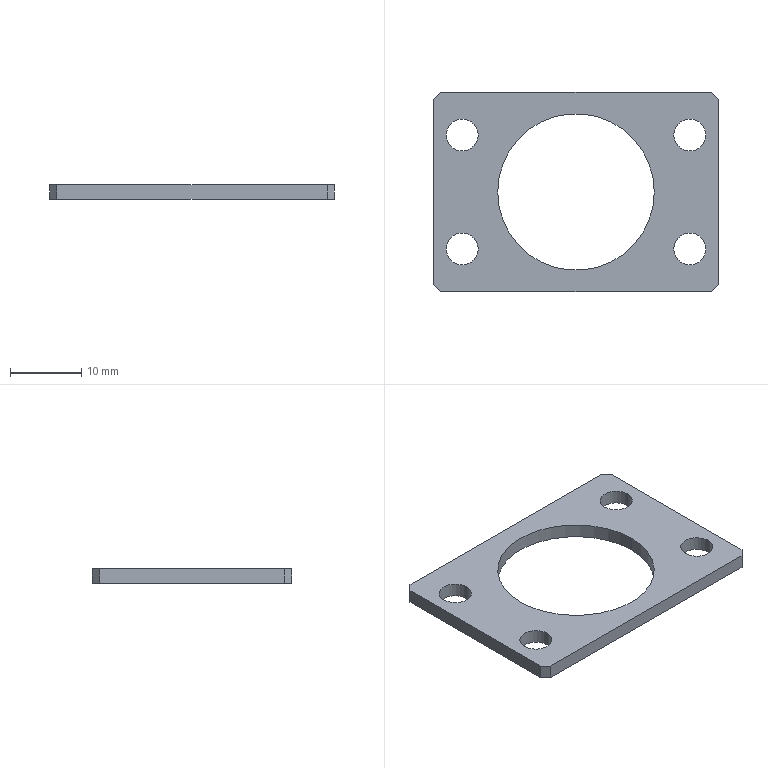Part | STEP file | 6001Z bearing stop plate | 1 solid | 20 faces | box 40 x 28 x 2 mm | volume 1349 mm3 | cylinder 10 | plane 10 | commonest cylinder face diameters 4.5 x8 22 x2
STEP:
#1=CARTESIAN_POINT('',(0.,0.,0.));
#2=DIRECTION('',(0.,0.,1.));
#3=DIRECTION('',(1.,0.,0.));
#4=AXIS2_PLACEMENT_3D('',#1,#2,#3);
#5=CARTESIAN_POINT('',(18.25,8.,-2.));
#6=VERTEX_POINT('',#5);
#7=CARTESIAN_POINT('',(18.25,8.,0.));
#8=VERTEX_POINT('',#7);
#9=CARTESIAN_POINT('',(18.25,8.,0.));
#10=DIRECTION('',(0.,0.,1.));
#11=VECTOR('',#10,1.);
#12=LINE('',#9,#11);
#13=CARTESIAN_POINT('',(16.,8.,0.));
#14=DIRECTION('',(0.,0.,1.));
#15=DIRECTION('',(1.,0.,0.));
#16=AXIS2_PLACEMENT_3D('',#13,#14,#15);
#17=CYLINDRICAL_SURFACE('',#16,2.25);
#18=CARTESIAN_POINT('',(6.283,0.));
#19=DIRECTION('',(0.,1.));
#20=VECTOR('',#19,1.);
#21=LINE('',#18,#20);
#22=(GEOMETRIC_REPRESENTATION_CONTEXT(2)PARAMETRIC_REPRESENTATION_CONTEXT()REPRESENTATION_CONTEXT('',''));
#23=DEFINITIONAL_REPRESENTATION('',(#21),#22);
#24=PCURVE('',#17,#23);
#25=CARTESIAN_POINT('',(16.,8.,0.));
#26=DIRECTION('',(0.,0.,1.));
#27=DIRECTION('',(1.,0.,0.));
#28=AXIS2_PLACEMENT_3D('',#25,#26,#27);
#29=CYLINDRICAL_SURFACE('',#28,2.25);
#30=CARTESIAN_POINT('',(0.,0.));
#31=DIRECTION('',(0.,1.));
#32=VECTOR('',#31,1.);
#33=LINE('',#30,#32);
#34=(GEOMETRIC_REPRESENTATION_CONTEXT(2)PARAMETRIC_REPRESENTATION_CONTEXT()REPRESENTATION_CONTEXT('',''));
#35=DEFINITIONAL_REPRESENTATION('',(#33),#34);
#36=PCURVE('',#29,#35);
#37=SURFACE_CURVE('',#12,(#24,#36),.PCURVE_S1.);
#38=EDGE_CURVE('',#6,#8,#37,.T.);
#39=ORIENTED_EDGE('',*,*,#38,.T.);
#40=CARTESIAN_POINT('',(13.75,8.,0.));
#41=VERTEX_POINT('',#40);
#42=CARTESIAN_POINT('',(16.,8.,0.));
#43=DIRECTION('',(0.,0.,1.));
#44=DIRECTION('',(1.,0.,0.));
#45=AXIS2_PLACEMENT_3D('',#42,#43,#44);
#46=CIRCLE('',#45,2.25);
#47=CARTESIAN_POINT('',(0.,0.));
#48=DIRECTION('',(1.,0.));
#49=VECTOR('',#48,1.);
#50=LINE('',#47,#49);
#51=(GEOMETRIC_REPRESENTATION_CONTEXT(2)PARAMETRIC_REPRESENTATION_CONTEXT()REPRESENTATION_CONTEXT('',''));
#52=DEFINITIONAL_REPRESENTATION('',(#50),#51);
#53=PCURVE('',#17,#52);
#54=CARTESIAN_POINT('',(20.,-14.,0.));
#55=DIRECTION('',(0.,0.,1.));
#56=DIRECTION('',(1.,0.,0.));
#57=AXIS2_PLACEMENT_3D('',#54,#55,#56);
#58=PLANE('',#57);
#59=CARTESIAN_POINT('',(-4.,22.));
#60=DIRECTION('',(1.,0.));
#61=AXIS2_PLACEMENT_2D('',#59,#60);
#62=CIRCLE('',#61,2.25);
#63=(GEOMETRIC_REPRESENTATION_CONTEXT(2)PARAMETRIC_REPRESENTATION_CONTEXT()REPRESENTATION_CONTEXT('',''));
#64=DEFINITIONAL_REPRESENTATION('',(#62),#63);
#65=PCURVE('',#58,#64);
#66=SURFACE_CURVE('',#46,(#53,#65),.PCURVE_S1.);
#67=EDGE_CURVE('',#41,#8,#66,.T.);
#68=ORIENTED_EDGE('',*,*,#67,.F.);
#69=CARTESIAN_POINT('',(13.75,8.,-2.));
#70=VERTEX_POINT('',#69);
#71=CARTESIAN_POINT('',(13.75,8.,0.));
#72=DIRECTION('',(0.,0.,1.));
#73=VECTOR('',#72,1.);
#74=LINE('',#71,#73);
#75=CARTESIAN_POINT('',(3.142,0.));
#76=DIRECTION('',(0.,1.));
#77=VECTOR('',#76,1.);
#78=LINE('',#75,#77);
#79=(GEOMETRIC_REPRESENTATION_CONTEXT(2)PARAMETRIC_REPRESENTATION_CONTEXT()REPRESENTATION_CONTEXT('',''));
#80=DEFINITIONAL_REPRESENTATION('',(#78),#79);
#81=PCURVE('',#17,#80);
#82=CARTESIAN_POINT('',(3.142,0.));
#83=DIRECTION('',(0.,1.));
#84=VECTOR('',#83,1.);
#85=LINE('',#82,#84);
#86=(GEOMETRIC_REPRESENTATION_CONTEXT(2)PARAMETRIC_REPRESENTATION_CONTEXT()REPRESENTATION_CONTEXT('',''));
#87=DEFINITIONAL_REPRESENTATION('',(#85),#86);
#88=PCURVE('',#29,#87);
#89=SURFACE_CURVE('',#74,(#81,#88),.PCURVE_S1.);
#90=EDGE_CURVE('',#70,#41,#89,.T.);
#91=ORIENTED_EDGE('',*,*,#90,.F.);
#92=CARTESIAN_POINT('',(16.,8.,-2.));
#93=DIRECTION('',(0.,0.,1.));
#94=DIRECTION('',(1.,0.,0.));
#95=AXIS2_PLACEMENT_3D('',#92,#93,#94);
#96=CIRCLE('',#95,2.25);
#97=CARTESIAN_POINT('',(0.,-2.));
#98=DIRECTION('',(1.,0.));
#99=VECTOR('',#98,1.);
#100=LINE('',#97,#99);
#101=(GEOMETRIC_REPRESENTATION_CONTEXT(2)PARAMETRIC_REPRESENTATION_CONTEXT()REPRESENTATION_CONTEXT('',''));
#102=DEFINITIONAL_REPRESENTATION('',(#100),#101);
#103=PCURVE('',#17,#102);
#104=CARTESIAN_POINT('',(20.,-14.,-2.));
#105=DIRECTION('',(0.,0.,1.));
#106=DIRECTION('',(1.,0.,0.));
#107=AXIS2_PLACEMENT_3D('',#104,#105,#106);
#108=PLANE('',#107);
#109=CARTESIAN_POINT('',(-4.,22.));
#110=DIRECTION('',(1.,0.));
#111=AXIS2_PLACEMENT_2D('',#109,#110);
#112=CIRCLE('',#111,2.25);
#113=(GEOMETRIC_REPRESENTATION_CONTEXT(2)PARAMETRIC_REPRESENTATION_CONTEXT()REPRESENTATION_CONTEXT('',''));
#114=DEFINITIONAL_REPRESENTATION('',(#112),#113);
#115=PCURVE('',#108,#114);
#116=SURFACE_CURVE('',#96,(#103,#115),.PCURVE_S1.);
#117=EDGE_CURVE('',#70,#6,#116,.T.);
#118=ORIENTED_EDGE('',*,*,#117,.T.);
#119=EDGE_LOOP('',(#39,#68,#91,#118));
#120=FACE_BOUND('',#119,.F.);
#121=ADVANCED_FACE('',(#120),#17,.F.);
#122=CARTESIAN_POINT('',(-13.75,8.,-2.));
#123=VERTEX_POINT('',#122);
#124=CARTESIAN_POINT('',(-13.75,8.,0.));
#125=VERTEX_POINT('',#124);
#126=CARTESIAN_POINT('',(-13.75,8.,0.));
#127=DIRECTION('',(0.,0.,1.));
#128=VECTOR('',#127,1.);
#129=LINE('',#126,#128);
#130=CARTESIAN_POINT('',(-16.,8.,0.));
#131=DIRECTION('',(0.,0.,1.));
#132=DIRECTION('',(1.,0.,0.));
#133=AXIS2_PLACEMENT_3D('',#130,#131,#132);
#134=CYLINDRICAL_SURFACE('',#133,2.25);
#135=CARTESIAN_POINT('',(6.283,0.));
#136=DIRECTION('',(0.,1.));
#137=VECTOR('',#136,1.);
#138=LINE('',#135,#137);
#139=(GEOMETRIC_REPRESENTATION_CONTEXT(2)PARAMETRIC_REPRESENTATION_CONTEXT()REPRESENTATION_CONTEXT('',''));
#140=DEFINITIONAL_REPRESENTATION('',(#138),#139);
#141=PCURVE('',#134,#140);
#142=CARTESIAN_POINT('',(-16.,8.,0.));
#143=DIRECTION('',(0.,0.,1.));
#144=DIRECTION('',(1.,0.,0.));
#145=AXIS2_PLACEMENT_3D('',#142,#143,#144);
#146=CYLINDRICAL_SURFACE('',#145,2.25);
#147=CARTESIAN_POINT('',(0.,0.));
#148=DIRECTION('',(0.,1.));
#149=VECTOR('',#148,1.);
#150=LINE('',#147,#149);
#151=(GEOMETRIC_REPRESENTATION_CONTEXT(2)PARAMETRIC_REPRESENTATION_CONTEXT()REPRESENTATION_CONTEXT('',''));
#152=DEFINITIONAL_REPRESENTATION('',(#150),#151);
#153=PCURVE('',#146,#152);
#154=SURFACE_CURVE('',#129,(#141,#153),.PCURVE_S1.);
#155=EDGE_CURVE('',#123,#125,#154,.T.);
#156=ORIENTED_EDGE('',*,*,#155,.T.);
#157=CARTESIAN_POINT('',(-18.25,8.,0.));
#158=VERTEX_POINT('',#157);
#159=CARTESIAN_POINT('',(-16.,8.,0.));
#160=DIRECTION('',(0.,0.,1.));
#161=DIRECTION('',(1.,0.,0.));
#162=AXIS2_PLACEMENT_3D('',#159,#160,#161);
#163=CIRCLE('',#162,2.25);
#164=CARTESIAN_POINT('',(0.,0.));
#165=DIRECTION('',(1.,0.));
#166=VECTOR('',#165,1.);
#167=LINE('',#164,#166);
#168=(GEOMETRIC_REPRESENTATION_CONTEXT(2)PARAMETRIC_REPRESENTATION_CONTEXT()REPRESENTATION_CONTEXT('',''));
#169=DEFINITIONAL_REPRESENTATION('',(#167),#168);
#170=PCURVE('',#134,#169);
#171=CARTESIAN_POINT('',(-36.,22.));
#172=DIRECTION('',(1.,0.));
#173=AXIS2_PLACEMENT_2D('',#171,#172);
#174=CIRCLE('',#173,2.25);
#175=(GEOMETRIC_REPRESENTATION_CONTEXT(2)PARAMETRIC_REPRESENTATION_CONTEXT()REPRESENTATION_CONTEXT('',''));
#176=DEFINITIONAL_REPRESENTATION('',(#174),#175);
#177=PCURVE('',#58,#176);
#178=SURFACE_CURVE('',#163,(#170,#177),.PCURVE_S1.);
#179=EDGE_CURVE('',#158,#125,#178,.T.);
#180=ORIENTED_EDGE('',*,*,#179,.F.);
#181=CARTESIAN_POINT('',(-18.25,8.,-2.));
#182=VERTEX_POINT('',#181);
#183=CARTESIAN_POINT('',(-18.25,8.,0.));
#184=DIRECTION('',(0.,0.,1.));
#185=VECTOR('',#184,1.);
#186=LINE('',#183,#185);
#187=CARTESIAN_POINT('',(3.142,0.));
#188=DIRECTION('',(0.,1.));
#189=VECTOR('',#188,1.);
#190=LINE('',#187,#189);
#191=(GEOMETRIC_REPRESENTATION_CONTEXT(2)PARAMETRIC_REPRESENTATION_CONTEXT()REPRESENTATION_CONTEXT('',''));
#192=DEFINITIONAL_REPRESENTATION('',(#190),#191);
#193=PCURVE('',#134,#192);
#194=CARTESIAN_POINT('',(3.142,0.));
#195=DIRECTION('',(0.,1.));
#196=VECTOR('',#195,1.);
#197=LINE('',#194,#196);
#198=(GEOMETRIC_REPRESENTATION_CONTEXT(2)PARAMETRIC_REPRESENTATION_CONTEXT()REPRESENTATION_CONTEXT('',''));
#199=DEFINITIONAL_REPRESENTATION('',(#197),#198);
#200=PCURVE('',#146,#199);
#201=SURFACE_CURVE('',#186,(#193,#200),.PCURVE_S1.);
#202=EDGE_CURVE('',#182,#158,#201,.T.);
#203=ORIENTED_EDGE('',*,*,#202,.F.);
#204=CARTESIAN_POINT('',(-16.,8.,-2.));
#205=DIRECTION('',(0.,0.,1.));
#206=DIRECTION('',(1.,0.,0.));
#207=AXIS2_PLACEMENT_3D('',#204,#205,#206);
#208=CIRCLE('',#207,2.25);
#209=CARTESIAN_POINT('',(0.,-2.));
#210=DIRECTION('',(1.,0.));
#211=VECTOR('',#210,1.);
#212=LINE('',#209,#211);
#213=(GEOMETRIC_REPRESENTATION_CONTEXT(2)PARAMETRIC_REPRESENTATION_CONTEXT()REPRESENTATION_CONTEXT('',''));
#214=DEFINITIONAL_REPRESENTATION('',(#212),#213);
#215=PCURVE('',#134,#214);
#216=CARTESIAN_POINT('',(-36.,22.));
#217=DIRECTION('',(1.,0.));
#218=AXIS2_PLACEMENT_2D('',#216,#217);
#219=CIRCLE('',#218,2.25);
#220=(GEOMETRIC_REPRESENTATION_CONTEXT(2)PARAMETRIC_REPRESENTATION_CONTEXT()REPRESENTATION_CONTEXT('',''));
#221=DEFINITIONAL_REPRESENTATION('',(#219),#220);
#222=PCURVE('',#108,#221);
#223=SURFACE_CURVE('',#208,(#215,#222),.PCURVE_S1.);
#224=EDGE_CURVE('',#182,#123,#223,.T.);
#225=ORIENTED_EDGE('',*,*,#224,.T.);
#226=EDGE_LOOP('',(#156,#180,#203,#225));
#227=FACE_BOUND('',#226,.F.);
#228=ADVANCED_FACE('',(#227),#134,.F.);
#229=CARTESIAN_POINT('',(-13.75,-8.,-2.));
#230=VERTEX_POINT('',#229);
#231=CARTESIAN_POINT('',(-13.75,-8.,0.));
#232=VERTEX_POINT('',#231);
#233=CARTESIAN_POINT('',(-13.75,-8.,0.));
#234=DIRECTION('',(0.,0.,1.));
#235=VECTOR('',#234,1.);
#236=LINE('',#233,#235);
#237=CARTESIAN_POINT('',(-16.,-8.,0.));
#238=DIRECTION('',(0.,0.,1.));
#239=DIRECTION('',(1.,0.,0.));
#240=AXIS2_PLACEMENT_3D('',#237,#238,#239);
#241=CYLINDRICAL_SURFACE('',#240,2.25);
#242=CARTESIAN_POINT('',(6.283,0.));
#243=DIRECTION('',(0.,1.));
#244=VECTOR('',#243,1.);
#245=LINE('',#242,#244);
#246=(GEOMETRIC_REPRESENTATION_CONTEXT(2)PARAMETRIC_REPRESENTATION_CONTEXT()REPRESENTATION_CONTEXT('',''));
#247=DEFINITIONAL_REPRESENTATION('',(#245),#246);
#248=PCURVE('',#241,#247);
#249=CARTESIAN_POINT('',(-16.,-8.,0.));
#250=DIRECTION('',(0.,0.,1.));
#251=DIRECTION('',(1.,0.,0.));
#252=AXIS2_PLACEMENT_3D('',#249,#250,#251);
#253=CYLINDRICAL_SURFACE('',#252,2.25);
#254=CARTESIAN_POINT('',(0.,0.));
#255=DIRECTION('',(0.,1.));
#256=VECTOR('',#255,1.);
#257=LINE('',#254,#256);
#258=(GEOMETRIC_REPRESENTATION_CONTEXT(2)PARAMETRIC_REPRESENTATION_CONTEXT()REPRESENTATION_CONTEXT('',''));
#259=DEFINITIONAL_REPRESENTATION('',(#257),#258);
#260=PCURVE('',#253,#259);
#261=SURFACE_CURVE('',#236,(#248,#260),.PCURVE_S1.);
#262=EDGE_CURVE('',#230,#232,#261,.T.);
#263=ORIENTED_EDGE('',*,*,#262,.T.);
#264=CARTESIAN_POINT('',(-18.25,-8.,0.));
#265=VERTEX_POINT('',#264);
#266=CARTESIAN_POINT('',(-16.,-8.,0.));
#267=DIRECTION('',(0.,0.,1.));
#268=DIRECTION('',(1.,0.,0.));
#269=AXIS2_PLACEMENT_3D('',#266,#267,#268);
#270=CIRCLE('',#269,2.25);
#271=CARTESIAN_POINT('',(0.,0.));
#272=DIRECTION('',(1.,0.));
#273=VECTOR('',#272,1.);
#274=LINE('',#271,#273);
#275=(GEOMETRIC_REPRESENTATION_CONTEXT(2)PARAMETRIC_REPRESENTATION_CONTEXT()REPRESENTATION_CONTEXT('',''));
#276=DEFINITIONAL_REPRESENTATION('',(#274),#275);
#277=PCURVE('',#241,#276);
#278=CARTESIAN_POINT('',(-36.,6.));
#279=DIRECTION('',(1.,0.));
#280=AXIS2_PLACEMENT_2D('',#278,#279);
#281=CIRCLE('',#280,2.25);
#282=(GEOMETRIC_REPRESENTATION_CONTEXT(2)PARAMETRIC_REPRESENTATION_CONTEXT()REPRESENTATION_CONTEXT('',''));
#283=DEFINITIONAL_REPRESENTATION('',(#281),#282);
#284=PCURVE('',#58,#283);
#285=SURFACE_CURVE('',#270,(#277,#284),.PCURVE_S1.);
#286=EDGE_CURVE('',#265,#232,#285,.T.);
#287=ORIENTED_EDGE('',*,*,#286,.F.);
#288=CARTESIAN_POINT('',(-18.25,-8.,-2.));
#289=VERTEX_POINT('',#288);
#290=CARTESIAN_POINT('',(-18.25,-8.,0.));
#291=DIRECTION('',(0.,0.,1.));
#292=VECTOR('',#291,1.);
#293=LINE('',#290,#292);
#294=CARTESIAN_POINT('',(3.142,0.));
#295=DIRECTION('',(0.,1.));
#296=VECTOR('',#295,1.);
#297=LINE('',#294,#296);
#298=(GEOMETRIC_REPRESENTATION_CONTEXT(2)PARAMETRIC_REPRESENTATION_CONTEXT()REPRESENTATION_CONTEXT('',''));
#299=DEFINITIONAL_REPRESENTATION('',(#297),#298);
#300=PCURVE('',#241,#299);
#301=CARTESIAN_POINT('',(3.142,0.));
#302=DIRECTION('',(0.,1.));
#303=VECTOR('',#302,1.);
#304=LINE('',#301,#303);
#305=(GEOMETRIC_REPRESENTATION_CONTEXT(2)PARAMETRIC_REPRESENTATION_CONTEXT()REPRESENTATION_CONTEXT('',''));
#306=DEFINITIONAL_REPRESENTATION('',(#304),#305);
#307=PCURVE('',#253,#306);
#308=SURFACE_CURVE('',#293,(#300,#307),.PCURVE_S1.);
#309=EDGE_CURVE('',#289,#265,#308,.T.);
#310=ORIENTED_EDGE('',*,*,#309,.F.);
#311=CARTESIAN_POINT('',(-16.,-8.,-2.));
#312=DIRECTION('',(0.,0.,1.));
#313=DIRECTION('',(1.,0.,0.));
#314=AXIS2_PLACEMENT_3D('',#311,#312,#313);
#315=CIRCLE('',#314,2.25);
#316=CARTESIAN_POINT('',(0.,-2.));
#317=DIRECTION('',(1.,0.));
#318=VECTOR('',#317,1.);
#319=LINE('',#316,#318);
#320=(GEOMETRIC_REPRESENTATION_CONTEXT(2)PARAMETRIC_REPRESENTATION_CONTEXT()REPRESENTATION_CONTEXT('',''));
#321=DEFINITIONAL_REPRESENTATION('',(#319),#320);
#322=PCURVE('',#241,#321);
#323=CARTESIAN_POINT('',(-36.,6.));
#324=DIRECTION('',(1.,0.));
#325=AXIS2_PLACEMENT_2D('',#323,#324);
#326=CIRCLE('',#325,2.25);
#327=(GEOMETRIC_REPRESENTATION_CONTEXT(2)PARAMETRIC_REPRESENTATION_CONTEXT()REPRESENTATION_CONTEXT('',''));
#328=DEFINITIONAL_REPRESENTATION('',(#326),#327);
#329=PCURVE('',#108,#328);
#330=SURFACE_CURVE('',#315,(#322,#329),.PCURVE_S1.);
#331=EDGE_CURVE('',#289,#230,#330,.T.);
#332=ORIENTED_EDGE('',*,*,#331,.T.);
#333=EDGE_LOOP('',(#263,#287,#310,#332));
#334=FACE_BOUND('',#333,.F.);
#335=ADVANCED_FACE('',(#334),#241,.F.);
#336=CARTESIAN_POINT('',(18.25,-8.,-2.));
#337=VERTEX_POINT('',#336);
#338=CARTESIAN_POINT('',(18.25,-8.,0.));
#339=VERTEX_POINT('',#338);
#340=CARTESIAN_POINT('',(18.25,-8.,0.));
#341=DIRECTION('',(0.,0.,1.));
#342=VECTOR('',#341,1.);
#343=LINE('',#340,#342);
#344=CARTESIAN_POINT('',(16.,-8.,0.));
#345=DIRECTION('',(0.,0.,1.));
#346=DIRECTION('',(1.,0.,0.));
#347=AXIS2_PLACEMENT_3D('',#344,#345,#346);
#348=CYLINDRICAL_SURFACE('',#347,2.25);
#349=CARTESIAN_POINT('',(6.283,0.));
#350=DIRECTION('',(0.,1.));
#351=VECTOR('',#350,1.);
#352=LINE('',#349,#351);
#353=(GEOMETRIC_REPRESENTATION_CONTEXT(2)PARAMETRIC_REPRESENTATION_CONTEXT()REPRESENTATION_CONTEXT('',''));
#354=DEFINITIONAL_REPRESENTATION('',(#352),#353);
#355=PCURVE('',#348,#354);
#356=CARTESIAN_POINT('',(16.,-8.,0.));
#357=DIRECTION('',(0.,0.,1.));
#358=DIRECTION('',(1.,0.,0.));
#359=AXIS2_PLACEMENT_3D('',#356,#357,#358);
#360=CYLINDRICAL_SURFACE('',#359,2.25);
#361=CARTESIAN_POINT('',(0.,0.));
#362=DIRECTION('',(0.,1.));
#363=VECTOR('',#362,1.);
#364=LINE('',#361,#363);
#365=(GEOMETRIC_REPRESENTATION_CONTEXT(2)PARAMETRIC_REPRESENTATION_CONTEXT()REPRESENTATION_CONTEXT('',''));
#366=DEFINITIONAL_REPRESENTATION('',(#364),#365);
#367=PCURVE('',#360,#366);
#368=SURFACE_CURVE('',#343,(#355,#367),.PCURVE_S1.);
#369=EDGE_CURVE('',#337,#339,#368,.T.);
#370=ORIENTED_EDGE('',*,*,#369,.T.);
#371=CARTESIAN_POINT('',(13.75,-8.,0.));
#372=VERTEX_POINT('',#371);
#373=CARTESIAN_POINT('',(16.,-8.,0.));
#374=DIRECTION('',(0.,0.,1.));
#375=DIRECTION('',(1.,0.,0.));
#376=AXIS2_PLACEMENT_3D('',#373,#374,#375);
#377=CIRCLE('',#376,2.25);
#378=CARTESIAN_POINT('',(0.,0.));
#379=DIRECTION('',(1.,0.));
#380=VECTOR('',#379,1.);
#381=LINE('',#378,#380);
#382=(GEOMETRIC_REPRESENTATION_CONTEXT(2)PARAMETRIC_REPRESENTATION_CONTEXT()REPRESENTATION_CONTEXT('',''));
#383=DEFINITIONAL_REPRESENTATION('',(#381),#382);
#384=PCURVE('',#348,#383);
#385=CARTESIAN_POINT('',(-4.,6.));
#386=DIRECTION('',(1.,0.));
#387=AXIS2_PLACEMENT_2D('',#385,#386);
#388=CIRCLE('',#387,2.25);
#389=(GEOMETRIC_REPRESENTATION_CONTEXT(2)PARAMETRIC_REPRESENTATION_CONTEXT()REPRESENTATION_CONTEXT('',''));
#390=DEFINITIONAL_REPRESENTATION('',(#388),#389);
#391=PCURVE('',#58,#390);
#392=SURFACE_CURVE('',#377,(#384,#391),.PCURVE_S1.);
#393=EDGE_CURVE('',#372,#339,#392,.T.);
#394=ORIENTED_EDGE('',*,*,#393,.F.);
#395=CARTESIAN_POINT('',(13.75,-8.,-2.));
#396=VERTEX_POINT('',#395);
#397=CARTESIAN_POINT('',(13.75,-8.,0.));
#398=DIRECTION('',(0.,0.,1.));
#399=VECTOR('',#398,1.);
#400=LINE('',#397,#399);
#401=CARTESIAN_POINT('',(3.142,0.));
#402=DIRECTION('',(0.,1.));
#403=VECTOR('',#402,1.);
#404=LINE('',#401,#403);
#405=(GEOMETRIC_REPRESENTATION_CONTEXT(2)PARAMETRIC_REPRESENTATION_CONTEXT()REPRESENTATION_CONTEXT('',''));
#406=DEFINITIONAL_REPRESENTATION('',(#404),#405);
#407=PCURVE('',#348,#406);
#408=CARTESIAN_POINT('',(3.142,0.));
#409=DIRECTION('',(0.,1.));
#410=VECTOR('',#409,1.);
#411=LINE('',#408,#410);
#412=(GEOMETRIC_REPRESENTATION_CONTEXT(2)PARAMETRIC_REPRESENTATION_CONTEXT()REPRESENTATION_CONTEXT('',''));
#413=DEFINITIONAL_REPRESENTATION('',(#411),#412);
#414=PCURVE('',#360,#413);
#415=SURFACE_CURVE('',#400,(#407,#414),.PCURVE_S1.);
#416=EDGE_CURVE('',#396,#372,#415,.T.);
#417=ORIENTED_EDGE('',*,*,#416,.F.);
#418=CARTESIAN_POINT('',(16.,-8.,-2.));
#419=DIRECTION('',(0.,0.,1.));
#420=DIRECTION('',(1.,0.,0.));
#421=AXIS2_PLACEMENT_3D('',#418,#419,#420);
#422=CIRCLE('',#421,2.25);
#423=CARTESIAN_POINT('',(0.,-2.));
#424=DIRECTION('',(1.,0.));
#425=VECTOR('',#424,1.);
#426=LINE('',#423,#425);
#427=(GEOMETRIC_REPRESENTATION_CONTEXT(2)PARAMETRIC_REPRESENTATION_CONTEXT()REPRESENTATION_CONTEXT('',''));
#428=DEFINITIONAL_REPRESENTATION('',(#426),#427);
#429=PCURVE('',#348,#428);
#430=CARTESIAN_POINT('',(-4.,6.));
#431=DIRECTION('',(1.,0.));
#432=AXIS2_PLACEMENT_2D('',#430,#431);
#433=CIRCLE('',#432,2.25);
#434=(GEOMETRIC_REPRESENTATION_CONTEXT(2)PARAMETRIC_REPRESENTATION_CONTEXT()REPRESENTATION_CONTEXT('',''));
#435=DEFINITIONAL_REPRESENTATION('',(#433),#434);
#436=PCURVE('',#108,#435);
#437=SURFACE_CURVE('',#422,(#429,#436),.PCURVE_S1.);
#438=EDGE_CURVE('',#396,#337,#437,.T.);
#439=ORIENTED_EDGE('',*,*,#438,.T.);
#440=EDGE_LOOP('',(#370,#394,#417,#439));
#441=FACE_BOUND('',#440,.F.);
#442=ADVANCED_FACE('',(#441),#348,.F.);
#443=CARTESIAN_POINT('',(11.,0.,-2.));
#444=VERTEX_POINT('',#443);
#445=CARTESIAN_POINT('',(11.,0.,0.));
#446=VERTEX_POINT('',#445);
#447=CARTESIAN_POINT('',(11.,0.,-2.));
#448=DIRECTION('',(0.,0.,1.));
#449=VECTOR('',#448,1.);
#450=LINE('',#447,#449);
#451=CARTESIAN_POINT('',(0.,0.,-2.));
#452=DIRECTION('',(0.,0.,1.));
#453=DIRECTION('',(1.,0.,0.));
#454=AXIS2_PLACEMENT_3D('',#451,#452,#453);
#455=CYLINDRICAL_SURFACE('',#454,11.);
#456=CARTESIAN_POINT('',(6.283,0.));
#457=DIRECTION('',(0.,1.));
#458=VECTOR('',#457,1.);
#459=LINE('',#456,#458);
#460=(GEOMETRIC_REPRESENTATION_CONTEXT(2)PARAMETRIC_REPRESENTATION_CONTEXT()REPRESENTATION_CONTEXT('',''));
#461=DEFINITIONAL_REPRESENTATION('',(#459),#460);
#462=PCURVE('',#455,#461);
#463=CARTESIAN_POINT('',(0.,0.,-2.));
#464=DIRECTION('',(0.,0.,1.));
#465=DIRECTION('',(1.,0.,0.));
#466=AXIS2_PLACEMENT_3D('',#463,#464,#465);
#467=CYLINDRICAL_SURFACE('',#466,11.);
#468=CARTESIAN_POINT('',(0.,0.));
#469=DIRECTION('',(0.,1.));
#470=VECTOR('',#469,1.);
#471=LINE('',#468,#470);
#472=(GEOMETRIC_REPRESENTATION_CONTEXT(2)PARAMETRIC_REPRESENTATION_CONTEXT()REPRESENTATION_CONTEXT('',''));
#473=DEFINITIONAL_REPRESENTATION('',(#471),#472);
#474=PCURVE('',#467,#473);
#475=SURFACE_CURVE('',#450,(#462,#474),.PCURVE_S1.);
#476=EDGE_CURVE('',#444,#446,#475,.T.);
#477=ORIENTED_EDGE('',*,*,#476,.T.);
#478=CARTESIAN_POINT('',(-11.,0.,0.));
#479=VERTEX_POINT('',#478);
#480=CARTESIAN_POINT('',(0.,0.,0.));
#481=DIRECTION('',(0.,0.,1.));
#482=DIRECTION('',(1.,0.,0.));
#483=AXIS2_PLACEMENT_3D('',#480,#481,#482);
#484=CIRCLE('',#483,11.);
#485=CARTESIAN_POINT('',(0.,2.));
#486=DIRECTION('',(1.,0.));
#487=VECTOR('',#486,1.);
#488=LINE('',#485,#487);
#489=(GEOMETRIC_REPRESENTATION_CONTEXT(2)PARAMETRIC_REPRESENTATION_CONTEXT()REPRESENTATION_CONTEXT('',''));
#490=DEFINITIONAL_REPRESENTATION('',(#488),#489);
#491=PCURVE('',#455,#490);
#492=CARTESIAN_POINT('',(-20.,14.));
#493=DIRECTION('',(1.,0.));
#494=AXIS2_PLACEMENT_2D('',#492,#493);
#495=CIRCLE('',#494,11.);
#496=(GEOMETRIC_REPRESENTATION_CONTEXT(2)PARAMETRIC_REPRESENTATION_CONTEXT()REPRESENTATION_CONTEXT('',''));
#497=DEFINITIONAL_REPRESENTATION('',(#495),#496);
#498=PCURVE('',#58,#497);
#499=SURFACE_CURVE('',#484,(#491,#498),.PCURVE_S1.);
#500=EDGE_CURVE('',#479,#446,#499,.T.);
#501=ORIENTED_EDGE('',*,*,#500,.F.);
#502=CARTESIAN_POINT('',(-11.,0.,-2.));
#503=VERTEX_POINT('',#502);
#504=CARTESIAN_POINT('',(-11.,0.,-2.));
#505=DIRECTION('',(0.,0.,1.));
#506=VECTOR('',#505,1.);
#507=LINE('',#504,#506);
#508=CARTESIAN_POINT('',(3.142,0.));
#509=DIRECTION('',(0.,1.));
#510=VECTOR('',#509,1.);
#511=LINE('',#508,#510);
#512=(GEOMETRIC_REPRESENTATION_CONTEXT(2)PARAMETRIC_REPRESENTATION_CONTEXT()REPRESENTATION_CONTEXT('',''));
#513=DEFINITIONAL_REPRESENTATION('',(#511),#512);
#514=PCURVE('',#455,#513);
#515=CARTESIAN_POINT('',(3.142,0.));
#516=DIRECTION('',(0.,1.));
#517=VECTOR('',#516,1.);
#518=LINE('',#515,#517);
#519=(GEOMETRIC_REPRESENTATION_CONTEXT(2)PARAMETRIC_REPRESENTATION_CONTEXT()REPRESENTATION_CONTEXT('',''));
#520=DEFINITIONAL_REPRESENTATION('',(#518),#519);
#521=PCURVE('',#467,#520);
#522=SURFACE_CURVE('',#507,(#514,#521),.PCURVE_S1.);
#523=EDGE_CURVE('',#503,#479,#522,.T.);
#524=ORIENTED_EDGE('',*,*,#523,.F.);
#525=CARTESIAN_POINT('',(0.,0.,-2.));
#526=DIRECTION('',(0.,0.,1.));
#527=DIRECTION('',(1.,0.,0.));
#528=AXIS2_PLACEMENT_3D('',#525,#526,#527);
#529=CIRCLE('',#528,11.);
#530=CARTESIAN_POINT('',(0.,0.));
#531=DIRECTION('',(1.,0.));
#532=VECTOR('',#531,1.);
#533=LINE('',#530,#532);
#534=(GEOMETRIC_REPRESENTATION_CONTEXT(2)PARAMETRIC_REPRESENTATION_CONTEXT()REPRESENTATION_CONTEXT('',''));
#535=DEFINITIONAL_REPRESENTATION('',(#533),#534);
#536=PCURVE('',#455,#535);
#537=CARTESIAN_POINT('',(-20.,14.));
#538=DIRECTION('',(1.,0.));
#539=AXIS2_PLACEMENT_2D('',#537,#538);
#540=CIRCLE('',#539,11.);
#541=(GEOMETRIC_REPRESENTATION_CONTEXT(2)PARAMETRIC_REPRESENTATION_CONTEXT()REPRESENTATION_CONTEXT('',''));
#542=DEFINITIONAL_REPRESENTATION('',(#540),#541);
#543=PCURVE('',#108,#542);
#544=SURFACE_CURVE('',#529,(#536,#543),.PCURVE_S1.);
#545=EDGE_CURVE('',#503,#444,#544,.T.);
#546=ORIENTED_EDGE('',*,*,#545,.T.);
#547=EDGE_LOOP('',(#477,#501,#524,#546));
#548=FACE_BOUND('',#547,.F.);
#549=ADVANCED_FACE('',(#548),#455,.F.);
#550=CARTESIAN_POINT('',(20.,-13.,0.));
#551=VERTEX_POINT('',#550);
#552=CARTESIAN_POINT('',(20.,13.,0.));
#553=VERTEX_POINT('',#552);
#554=CARTESIAN_POINT('',(20.,14.,0.));
#555=DIRECTION('',(0.,1.,0.));
#556=VECTOR('',#555,1.);
#557=LINE('',#554,#556);
#558=CARTESIAN_POINT('',(20.,14.,-2.));
#559=DIRECTION('',(1.,0.,0.));
#560=DIRECTION('',(0.,1.,0.));
#561=AXIS2_PLACEMENT_3D('',#558,#559,#560);
#562=PLANE('',#561);
#563=CARTESIAN_POINT('',(0.,2.));
#564=DIRECTION('',(1.,0.));
#565=VECTOR('',#564,1.);
#566=LINE('',#563,#565);
#567=(GEOMETRIC_REPRESENTATION_CONTEXT(2)PARAMETRIC_REPRESENTATION_CONTEXT()REPRESENTATION_CONTEXT('',''));
#568=DEFINITIONAL_REPRESENTATION('',(#566),#567);
#569=PCURVE('',#562,#568);
#570=CARTESIAN_POINT('',(0.,28.));
#571=DIRECTION('',(0.,1.));
#572=VECTOR('',#571,1.);
#573=LINE('',#570,#572);
#574=(GEOMETRIC_REPRESENTATION_CONTEXT(2)PARAMETRIC_REPRESENTATION_CONTEXT()REPRESENTATION_CONTEXT('',''));
#575=DEFINITIONAL_REPRESENTATION('',(#573),#574);
#576=PCURVE('',#58,#575);
#577=SURFACE_CURVE('',#557,(#569,#576),.PCURVE_S1.);
#578=EDGE_CURVE('',#551,#553,#577,.T.);
#579=ORIENTED_EDGE('',*,*,#578,.F.);
#580=CARTESIAN_POINT('',(20.,-13.,-2.));
#581=VERTEX_POINT('',#580);
#582=CARTESIAN_POINT('',(20.,-13.,-2.));
#583=DIRECTION('',(0.,0.,-1.));
#584=VECTOR('',#583,1.);
#585=LINE('',#582,#584);
#586=CARTESIAN_POINT('',(-27.,0.));
#587=DIRECTION('',(0.,-1.));
#588=VECTOR('',#587,1.);
#589=LINE('',#586,#588);
#590=(GEOMETRIC_REPRESENTATION_CONTEXT(2)PARAMETRIC_REPRESENTATION_CONTEXT()REPRESENTATION_CONTEXT('',''));
#591=DEFINITIONAL_REPRESENTATION('',(#589),#590);
#592=PCURVE('',#562,#591);
#593=CARTESIAN_POINT('',(19.,-14.,-2.));
#594=DIRECTION('',(-0.7071,0.7071,0.));
#595=DIRECTION('',(-0.7071,-0.7071,0.));
#596=AXIS2_PLACEMENT_3D('',#593,#594,#595);
#597=PLANE('',#596);
#598=CARTESIAN_POINT('',(-1.414,0.));
#599=DIRECTION('',(0.,-1.));
#600=VECTOR('',#599,1.);
#601=LINE('',#598,#600);
#602=(GEOMETRIC_REPRESENTATION_CONTEXT(2)PARAMETRIC_REPRESENTATION_CONTEXT()REPRESENTATION_CONTEXT('',''));
#603=DEFINITIONAL_REPRESENTATION('',(#601),#602);
#604=PCURVE('',#597,#603);
#605=SURFACE_CURVE('',#585,(#592,#604),.PCURVE_S1.);
#606=EDGE_CURVE('',#551,#581,#605,.T.);
#607=ORIENTED_EDGE('',*,*,#606,.T.);
#608=CARTESIAN_POINT('',(20.,13.,-2.));
#609=VERTEX_POINT('',#608);
#610=CARTESIAN_POINT('',(20.,14.,-2.));
#611=DIRECTION('',(0.,1.,0.));
#612=VECTOR('',#611,1.);
#613=LINE('',#610,#612);
#614=CARTESIAN_POINT('',(0.,0.));
#615=DIRECTION('',(1.,0.));
#616=VECTOR('',#615,1.);
#617=LINE('',#614,#616);
#618=(GEOMETRIC_REPRESENTATION_CONTEXT(2)PARAMETRIC_REPRESENTATION_CONTEXT()REPRESENTATION_CONTEXT('',''));
#619=DEFINITIONAL_REPRESENTATION('',(#617),#618);
#620=PCURVE('',#562,#619);
#621=CARTESIAN_POINT('',(0.,28.));
#622=DIRECTION('',(0.,1.));
#623=VECTOR('',#622,1.);
#624=LINE('',#621,#623);
#625=(GEOMETRIC_REPRESENTATION_CONTEXT(2)PARAMETRIC_REPRESENTATION_CONTEXT()REPRESENTATION_CONTEXT('',''));
#626=DEFINITIONAL_REPRESENTATION('',(#624),#625);
#627=PCURVE('',#108,#626);
#628=SURFACE_CURVE('',#613,(#620,#627),.PCURVE_S1.);
#629=EDGE_CURVE('',#581,#609,#628,.T.);
#630=ORIENTED_EDGE('',*,*,#629,.T.);
#631=CARTESIAN_POINT('',(20.,13.,-2.));
#632=DIRECTION('',(0.,0.,1.));
#633=VECTOR('',#632,1.);
#634=LINE('',#631,#633);
#635=CARTESIAN_POINT('',(-1.,0.));
#636=DIRECTION('',(0.,1.));
#637=VECTOR('',#636,1.);
#638=LINE('',#635,#637);
#639=(GEOMETRIC_REPRESENTATION_CONTEXT(2)PARAMETRIC_REPRESENTATION_CONTEXT()REPRESENTATION_CONTEXT('',''));
#640=DEFINITIONAL_REPRESENTATION('',(#638),#639);
#641=PCURVE('',#562,#640);
#642=CARTESIAN_POINT('',(20.,13.,-2.));
#643=DIRECTION('',(-0.7071,-0.7071,0.));
#644=DIRECTION('',(0.7071,-0.7071,0.));
#645=AXIS2_PLACEMENT_3D('',#642,#643,#644);
#646=PLANE('',#645);
#647=CARTESIAN_POINT('',(0.,0.));
#648=DIRECTION('',(0.,1.));
#649=VECTOR('',#648,1.);
#650=LINE('',#647,#649);
#651=(GEOMETRIC_REPRESENTATION_CONTEXT(2)PARAMETRIC_REPRESENTATION_CONTEXT()REPRESENTATION_CONTEXT('',''));
#652=DEFINITIONAL_REPRESENTATION('',(#650),#651);
#653=PCURVE('',#646,#652);
#654=SURFACE_CURVE('',#634,(#641,#653),.PCURVE_S1.);
#655=EDGE_CURVE('',#609,#553,#654,.T.);
#656=ORIENTED_EDGE('',*,*,#655,.T.);
#657=EDGE_LOOP('',(#579,#607,#630,#656));
#658=FACE_BOUND('',#657,.T.);
#659=ADVANCED_FACE('',(#658),#562,.T.);
#660=CARTESIAN_POINT('',(-19.,-14.,-2.));
#661=VERTEX_POINT('',#660);
#662=CARTESIAN_POINT('',(19.,-14.,-2.));
#663=VERTEX_POINT('',#662);
#664=CARTESIAN_POINT('',(-20.,-14.,-2.));
#665=DIRECTION('',(1.,0.,0.));
#666=VECTOR('',#665,1.);
#667=LINE('',#664,#666);
#668=CARTESIAN_POINT('',(-20.,-14.,-2.));
#669=DIRECTION('',(0.,-1.,0.));
#670=DIRECTION('',(0.,0.,-1.));
#671=AXIS2_PLACEMENT_3D('',#668,#669,#670);
#672=PLANE('',#671);
#673=CARTESIAN_POINT('',(0.,0.));
#674=DIRECTION('',(0.,1.));
#675=VECTOR('',#674,1.);
#676=LINE('',#673,#675);
#677=(GEOMETRIC_REPRESENTATION_CONTEXT(2)PARAMETRIC_REPRESENTATION_CONTEXT()REPRESENTATION_CONTEXT('',''));
#678=DEFINITIONAL_REPRESENTATION('',(#676),#677);
#679=PCURVE('',#672,#678);
#680=CARTESIAN_POINT('',(-40.,0.));
#681=DIRECTION('',(1.,0.));
#682=VECTOR('',#681,1.);
#683=LINE('',#680,#682);
#684=(GEOMETRIC_REPRESENTATION_CONTEXT(2)PARAMETRIC_REPRESENTATION_CONTEXT()REPRESENTATION_CONTEXT('',''));
#685=DEFINITIONAL_REPRESENTATION('',(#683),#684);
#686=PCURVE('',#108,#685);
#687=SURFACE_CURVE('',#667,(#679,#686),.PCURVE_S1.);
#688=EDGE_CURVE('',#661,#663,#687,.T.);
#689=ORIENTED_EDGE('',*,*,#688,.T.);
#690=CARTESIAN_POINT('',(19.,-14.,0.));
#691=VERTEX_POINT('',#690);
#692=CARTESIAN_POINT('',(19.,-14.,-2.));
#693=DIRECTION('',(0.,0.,1.));
#694=VECTOR('',#693,1.);
#695=LINE('',#692,#694);
#696=CARTESIAN_POINT('',(0.,39.));
#697=DIRECTION('',(-1.,0.));
#698=VECTOR('',#697,1.);
#699=LINE('',#696,#698);
#700=(GEOMETRIC_REPRESENTATION_CONTEXT(2)PARAMETRIC_REPRESENTATION_CONTEXT()REPRESENTATION_CONTEXT('',''));
#701=DEFINITIONAL_REPRESENTATION('',(#699),#700);
#702=PCURVE('',#672,#701);
#703=CARTESIAN_POINT('',(0.,0.));
#704=DIRECTION('',(0.,1.));
#705=VECTOR('',#704,1.);
#706=LINE('',#703,#705);
#707=(GEOMETRIC_REPRESENTATION_CONTEXT(2)PARAMETRIC_REPRESENTATION_CONTEXT()REPRESENTATION_CONTEXT('',''));
#708=DEFINITIONAL_REPRESENTATION('',(#706),#707);
#709=PCURVE('',#597,#708);
#710=SURFACE_CURVE('',#695,(#702,#709),.PCURVE_S1.);
#711=EDGE_CURVE('',#663,#691,#710,.T.);
#712=ORIENTED_EDGE('',*,*,#711,.T.);
#713=CARTESIAN_POINT('',(-19.,-14.,0.));
#714=VERTEX_POINT('',#713);
#715=CARTESIAN_POINT('',(-20.,-14.,0.));
#716=DIRECTION('',(1.,0.,0.));
#717=VECTOR('',#716,1.);
#718=LINE('',#715,#717);
#719=CARTESIAN_POINT('',(-2.,0.));
#720=DIRECTION('',(0.,1.));
#721=VECTOR('',#720,1.);
#722=LINE('',#719,#721);
#723=(GEOMETRIC_REPRESENTATION_CONTEXT(2)PARAMETRIC_REPRESENTATION_CONTEXT()REPRESENTATION_CONTEXT('',''));
#724=DEFINITIONAL_REPRESENTATION('',(#722),#723);
#725=PCURVE('',#672,#724);
#726=CARTESIAN_POINT('',(-40.,0.));
#727=DIRECTION('',(1.,0.));
#728=VECTOR('',#727,1.);
#729=LINE('',#726,#728);
#730=(GEOMETRIC_REPRESENTATION_CONTEXT(2)PARAMETRIC_REPRESENTATION_CONTEXT()REPRESENTATION_CONTEXT('',''));
#731=DEFINITIONAL_REPRESENTATION('',(#729),#730);
#732=PCURVE('',#58,#731);
#733=SURFACE_CURVE('',#718,(#725,#732),.PCURVE_S1.);
#734=EDGE_CURVE('',#714,#691,#733,.T.);
#735=ORIENTED_EDGE('',*,*,#734,.F.);
#736=CARTESIAN_POINT('',(-19.,-14.,-2.));
#737=DIRECTION('',(0.,0.,-1.));
#738=VECTOR('',#737,1.);
#739=LINE('',#736,#738);
#740=CARTESIAN_POINT('',(0.,1.));
#741=DIRECTION('',(1.,0.));
#742=VECTOR('',#741,1.);
#743=LINE('',#740,#742);
#744=(GEOMETRIC_REPRESENTATION_CONTEXT(2)PARAMETRIC_REPRESENTATION_CONTEXT()REPRESENTATION_CONTEXT('',''));
#745=DEFINITIONAL_REPRESENTATION('',(#743),#744);
#746=PCURVE('',#672,#745);
#747=CARTESIAN_POINT('',(-20.,-13.,-2.));
#748=DIRECTION('',(0.7071,0.7071,0.));
#749=DIRECTION('',(-0.7071,0.7071,0.));
#750=AXIS2_PLACEMENT_3D('',#747,#748,#749);
#751=PLANE('',#750);
#752=CARTESIAN_POINT('',(-1.414,0.));
#753=DIRECTION('',(0.,-1.));
#754=VECTOR('',#753,1.);
#755=LINE('',#752,#754);
#756=(GEOMETRIC_REPRESENTATION_CONTEXT(2)PARAMETRIC_REPRESENTATION_CONTEXT()REPRESENTATION_CONTEXT('',''));
#757=DEFINITIONAL_REPRESENTATION('',(#755),#756);
#758=PCURVE('',#751,#757);
#759=SURFACE_CURVE('',#739,(#746,#758),.PCURVE_S1.);
#760=EDGE_CURVE('',#714,#661,#759,.T.);
#761=ORIENTED_EDGE('',*,*,#760,.T.);
#762=EDGE_LOOP('',(#689,#712,#735,#761));
#763=FACE_BOUND('',#762,.T.);
#764=ADVANCED_FACE('',(#763),#672,.T.);
#765=CARTESIAN_POINT('',(-20.,13.,-2.));
#766=VERTEX_POINT('',#765);
#767=CARTESIAN_POINT('',(-20.,-13.,-2.));
#768=VERTEX_POINT('',#767);
#769=CARTESIAN_POINT('',(-20.,14.,-2.));
#770=DIRECTION('',(0.,-1.,0.));
#771=VECTOR('',#770,1.);
#772=LINE('',#769,#771);
#773=CARTESIAN_POINT('',(-20.,14.,-2.));
#774=DIRECTION('',(-1.,0.,0.));
#775=DIRECTION('',(0.,-1.,0.));
#776=AXIS2_PLACEMENT_3D('',#773,#774,#775);
#777=PLANE('',#776);
#778=CARTESIAN_POINT('',(0.,0.));
#779=DIRECTION('',(1.,0.));
#780=VECTOR('',#779,1.);
#781=LINE('',#778,#780);
#782=(GEOMETRIC_REPRESENTATION_CONTEXT(2)PARAMETRIC_REPRESENTATION_CONTEXT()REPRESENTATION_CONTEXT('',''));
#783=DEFINITIONAL_REPRESENTATION('',(#781),#782);
#784=PCURVE('',#777,#783);
#785=CARTESIAN_POINT('',(-40.,28.));
#786=DIRECTION('',(0.,-1.));
#787=VECTOR('',#786,1.);
#788=LINE('',#785,#787);
#789=(GEOMETRIC_REPRESENTATION_CONTEXT(2)PARAMETRIC_REPRESENTATION_CONTEXT()REPRESENTATION_CONTEXT('',''));
#790=DEFINITIONAL_REPRESENTATION('',(#788),#789);
#791=PCURVE('',#108,#790);
#792=SURFACE_CURVE('',#772,(#784,#791),.PCURVE_S1.);
#793=EDGE_CURVE('',#766,#768,#792,.T.);
#794=ORIENTED_EDGE('',*,*,#793,.T.);
#795=CARTESIAN_POINT('',(-20.,-13.,0.));
#796=VERTEX_POINT('',#795);
#797=CARTESIAN_POINT('',(-20.,-13.,-2.));
#798=DIRECTION('',(0.,0.,1.));
#799=VECTOR('',#798,1.);
#800=LINE('',#797,#799);
#801=CARTESIAN_POINT('',(27.,0.));
#802=DIRECTION('',(0.,1.));
#803=VECTOR('',#802,1.);
#804=LINE('',#801,#803);
#805=(GEOMETRIC_REPRESENTATION_CONTEXT(2)PARAMETRIC_REPRESENTATION_CONTEXT()REPRESENTATION_CONTEXT('',''));
#806=DEFINITIONAL_REPRESENTATION('',(#804),#805);
#807=PCURVE('',#777,#806);
#808=CARTESIAN_POINT('',(0.,0.));
#809=DIRECTION('',(0.,1.));
#810=VECTOR('',#809,1.);
#811=LINE('',#808,#810);
#812=(GEOMETRIC_REPRESENTATION_CONTEXT(2)PARAMETRIC_REPRESENTATION_CONTEXT()REPRESENTATION_CONTEXT('',''));
#813=DEFINITIONAL_REPRESENTATION('',(#811),#812);
#814=PCURVE('',#751,#813);
#815=SURFACE_CURVE('',#800,(#807,#814),.PCURVE_S1.);
#816=EDGE_CURVE('',#768,#796,#815,.T.);
#817=ORIENTED_EDGE('',*,*,#816,.T.);
#818=CARTESIAN_POINT('',(-20.,13.,0.));
#819=VERTEX_POINT('',#818);
#820=CARTESIAN_POINT('',(-20.,14.,0.));
#821=DIRECTION('',(0.,-1.,0.));
#822=VECTOR('',#821,1.);
#823=LINE('',#820,#822);
#824=CARTESIAN_POINT('',(0.,2.));
#825=DIRECTION('',(1.,0.));
#826=VECTOR('',#825,1.);
#827=LINE('',#824,#826);
#828=(GEOMETRIC_REPRESENTATION_CONTEXT(2)PARAMETRIC_REPRESENTATION_CONTEXT()REPRESENTATION_CONTEXT('',''));
#829=DEFINITIONAL_REPRESENTATION('',(#827),#828);
#830=PCURVE('',#777,#829);
#831=CARTESIAN_POINT('',(-40.,28.));
#832=DIRECTION('',(0.,-1.));
#833=VECTOR('',#832,1.);
#834=LINE('',#831,#833);
#835=(GEOMETRIC_REPRESENTATION_CONTEXT(2)PARAMETRIC_REPRESENTATION_CONTEXT()REPRESENTATION_CONTEXT('',''));
#836=DEFINITIONAL_REPRESENTATION('',(#834),#835);
#837=PCURVE('',#58,#836);
#838=SURFACE_CURVE('',#823,(#830,#837),.PCURVE_S1.);
#839=EDGE_CURVE('',#819,#796,#838,.T.);
#840=ORIENTED_EDGE('',*,*,#839,.F.);
#841=CARTESIAN_POINT('',(-20.,13.,-2.));
#842=DIRECTION('',(0.,0.,-1.));
#843=VECTOR('',#842,1.);
#844=LINE('',#841,#843);
#845=CARTESIAN_POINT('',(1.,0.));
#846=DIRECTION('',(0.,-1.));
#847=VECTOR('',#846,1.);
#848=LINE('',#845,#847);
#849=(GEOMETRIC_REPRESENTATION_CONTEXT(2)PARAMETRIC_REPRESENTATION_CONTEXT()REPRESENTATION_CONTEXT('',''));
#850=DEFINITIONAL_REPRESENTATION('',(#848),#849);
#851=PCURVE('',#777,#850);
#852=CARTESIAN_POINT('',(-19.,14.,-2.));
#853=DIRECTION('',(0.7071,-0.7071,0.));
#854=DIRECTION('',(0.7071,0.7071,0.));
#855=AXIS2_PLACEMENT_3D('',#852,#853,#854);
#856=PLANE('',#855);
#857=CARTESIAN_POINT('',(-1.414,0.));
#858=DIRECTION('',(0.,-1.));
#859=VECTOR('',#858,1.);
#860=LINE('',#857,#859);
#861=(GEOMETRIC_REPRESENTATION_CONTEXT(2)PARAMETRIC_REPRESENTATION_CONTEXT()REPRESENTATION_CONTEXT('',''));
#862=DEFINITIONAL_REPRESENTATION('',(#860),#861);
#863=PCURVE('',#856,#862);
#864=SURFACE_CURVE('',#844,(#851,#863),.PCURVE_S1.);
#865=EDGE_CURVE('',#819,#766,#864,.T.);
#866=ORIENTED_EDGE('',*,*,#865,.T.);
#867=EDGE_LOOP('',(#794,#817,#840,#866));
#868=FACE_BOUND('',#867,.T.);
#869=ADVANCED_FACE('',(#868),#777,.T.);
#870=CARTESIAN_POINT('',(19.,14.,0.));
#871=VERTEX_POINT('',#870);
#872=CARTESIAN_POINT('',(-19.,14.,0.));
#873=VERTEX_POINT('',#872);
#874=CARTESIAN_POINT('',(-20.,14.,0.));
#875=DIRECTION('',(-1.,0.,0.));
#876=VECTOR('',#875,1.);
#877=LINE('',#874,#876);
#878=CARTESIAN_POINT('',(-20.,14.,-2.));
#879=DIRECTION('',(0.,1.,0.));
#880=DIRECTION('',(0.,0.,1.));
#881=AXIS2_PLACEMENT_3D('',#878,#879,#880);
#882=PLANE('',#881);
#883=CARTESIAN_POINT('',(2.,0.));
#884=DIRECTION('',(0.,-1.));
#885=VECTOR('',#884,1.);
#886=LINE('',#883,#885);
#887=(GEOMETRIC_REPRESENTATION_CONTEXT(2)PARAMETRIC_REPRESENTATION_CONTEXT()REPRESENTATION_CONTEXT('',''));
#888=DEFINITIONAL_REPRESENTATION('',(#886),#887);
#889=PCURVE('',#882,#888);
#890=CARTESIAN_POINT('',(-40.,28.));
#891=DIRECTION('',(-1.,0.));
#892=VECTOR('',#891,1.);
#893=LINE('',#890,#892);
#894=(GEOMETRIC_REPRESENTATION_CONTEXT(2)PARAMETRIC_REPRESENTATION_CONTEXT()REPRESENTATION_CONTEXT('',''));
#895=DEFINITIONAL_REPRESENTATION('',(#893),#894);
#896=PCURVE('',#58,#895);
#897=SURFACE_CURVE('',#877,(#889,#896),.PCURVE_S1.);
#898=EDGE_CURVE('',#871,#873,#897,.T.);
#899=ORIENTED_EDGE('',*,*,#898,.F.);
#900=CARTESIAN_POINT('',(19.,14.,-2.));
#901=VERTEX_POINT('',#900);
#902=CARTESIAN_POINT('',(19.,14.,-2.));
#903=DIRECTION('',(0.,0.,-1.));
#904=VECTOR('',#903,1.);
#905=LINE('',#902,#904);
#906=CARTESIAN_POINT('',(0.,39.));
#907=DIRECTION('',(-1.,0.));
#908=VECTOR('',#907,1.);
#909=LINE('',#906,#908);
#910=(GEOMETRIC_REPRESENTATION_CONTEXT(2)PARAMETRIC_REPRESENTATION_CONTEXT()REPRESENTATION_CONTEXT('',''));
#911=DEFINITIONAL_REPRESENTATION('',(#909),#910);
#912=PCURVE('',#882,#911);
#913=CARTESIAN_POINT('',(-1.414,0.));
#914=DIRECTION('',(0.,-1.));
#915=VECTOR('',#914,1.);
#916=LINE('',#913,#915);
#917=(GEOMETRIC_REPRESENTATION_CONTEXT(2)PARAMETRIC_REPRESENTATION_CONTEXT()REPRESENTATION_CONTEXT('',''));
#918=DEFINITIONAL_REPRESENTATION('',(#916),#917);
#919=PCURVE('',#646,#918);
#920=SURFACE_CURVE('',#905,(#912,#919),.PCURVE_S1.);
#921=EDGE_CURVE('',#871,#901,#920,.T.);
#922=ORIENTED_EDGE('',*,*,#921,.T.);
#923=CARTESIAN_POINT('',(-19.,14.,-2.));
#924=VERTEX_POINT('',#923);
#925=CARTESIAN_POINT('',(-20.,14.,-2.));
#926=DIRECTION('',(-1.,0.,0.));
#927=VECTOR('',#926,1.);
#928=LINE('',#925,#927);
#929=CARTESIAN_POINT('',(0.,0.));
#930=DIRECTION('',(0.,-1.));
#931=VECTOR('',#930,1.);
#932=LINE('',#929,#931);
#933=(GEOMETRIC_REPRESENTATION_CONTEXT(2)PARAMETRIC_REPRESENTATION_CONTEXT()REPRESENTATION_CONTEXT('',''));
#934=DEFINITIONAL_REPRESENTATION('',(#932),#933);
#935=PCURVE('',#882,#934);
#936=CARTESIAN_POINT('',(-40.,28.));
#937=DIRECTION('',(-1.,0.));
#938=VECTOR('',#937,1.);
#939=LINE('',#936,#938);
#940=(GEOMETRIC_REPRESENTATION_CONTEXT(2)PARAMETRIC_REPRESENTATION_CONTEXT()REPRESENTATION_CONTEXT('',''));
#941=DEFINITIONAL_REPRESENTATION('',(#939),#940);
#942=PCURVE('',#108,#941);
#943=SURFACE_CURVE('',#928,(#935,#942),.PCURVE_S1.);
#944=EDGE_CURVE('',#901,#924,#943,.T.);
#945=ORIENTED_EDGE('',*,*,#944,.T.);
#946=CARTESIAN_POINT('',(-19.,14.,-2.));
#947=DIRECTION('',(0.,0.,1.));
#948=VECTOR('',#947,1.);
#949=LINE('',#946,#948);
#950=CARTESIAN_POINT('',(0.,1.));
#951=DIRECTION('',(1.,0.));
#952=VECTOR('',#951,1.);
#953=LINE('',#950,#952);
#954=(GEOMETRIC_REPRESENTATION_CONTEXT(2)PARAMETRIC_REPRESENTATION_CONTEXT()REPRESENTATION_CONTEXT('',''));
#955=DEFINITIONAL_REPRESENTATION('',(#953),#954);
#956=PCURVE('',#882,#955);
#957=CARTESIAN_POINT('',(0.,0.));
#958=DIRECTION('',(0.,1.));
#959=VECTOR('',#958,1.);
#960=LINE('',#957,#959);
#961=(GEOMETRIC_REPRESENTATION_CONTEXT(2)PARAMETRIC_REPRESENTATION_CONTEXT()REPRESENTATION_CONTEXT('',''));
#962=DEFINITIONAL_REPRESENTATION('',(#960),#961);
#963=PCURVE('',#856,#962);
#964=SURFACE_CURVE('',#949,(#956,#963),.PCURVE_S1.);
#965=EDGE_CURVE('',#924,#873,#964,.T.);
#966=ORIENTED_EDGE('',*,*,#965,.T.);
#967=EDGE_LOOP('',(#899,#922,#945,#966));
#968=FACE_BOUND('',#967,.T.);
#969=ADVANCED_FACE('',(#968),#882,.T.);
#970=CARTESIAN_POINT('',(16.,8.,-2.));
#971=DIRECTION('',(0.,0.,1.));
#972=DIRECTION('',(1.,0.,0.));
#973=AXIS2_PLACEMENT_3D('',#970,#971,#972);
#974=CIRCLE('',#973,2.25);
#975=CARTESIAN_POINT('',(-4.,22.));
#976=DIRECTION('',(1.,0.));
#977=AXIS2_PLACEMENT_2D('',#975,#976);
#978=CIRCLE('',#977,2.25);
#979=(GEOMETRIC_REPRESENTATION_CONTEXT(2)PARAMETRIC_REPRESENTATION_CONTEXT()REPRESENTATION_CONTEXT('',''));
#980=DEFINITIONAL_REPRESENTATION('',(#978),#979);
#981=PCURVE('',#108,#980);
#982=CARTESIAN_POINT('',(0.,-2.));
#983=DIRECTION('',(1.,0.));
#984=VECTOR('',#983,1.);
#985=LINE('',#982,#984);
#986=(GEOMETRIC_REPRESENTATION_CONTEXT(2)PARAMETRIC_REPRESENTATION_CONTEXT()REPRESENTATION_CONTEXT('',''));
#987=DEFINITIONAL_REPRESENTATION('',(#985),#986);
#988=PCURVE('',#29,#987);
#989=SURFACE_CURVE('',#974,(#981,#988),.PCURVE_S1.);
#990=EDGE_CURVE('',#6,#70,#989,.T.);
#991=ORIENTED_EDGE('',*,*,#990,.T.);
#992=ORIENTED_EDGE('',*,*,#117,.T.);
#993=EDGE_LOOP('',(#991,#992));
#994=FACE_BOUND('',#993,.T.);
#995=CARTESIAN_POINT('',(-16.,8.,-2.));
#996=DIRECTION('',(0.,0.,1.));
#997=DIRECTION('',(1.,0.,0.));
#998=AXIS2_PLACEMENT_3D('',#995,#996,#997);
#999=CIRCLE('',#998,2.25);
#1000=CARTESIAN_POINT('',(-36.,22.));
#1001=DIRECTION('',(1.,0.));
#1002=AXIS2_PLACEMENT_2D('',#1000,#1001);
#1003=CIRCLE('',#1002,2.25);
#1004=(GEOMETRIC_REPRESENTATION_CONTEXT(2)PARAMETRIC_REPRESENTATION_CONTEXT()REPRESENTATION_CONTEXT('',''));
#1005=DEFINITIONAL_REPRESENTATION('',(#1003),#1004);
#1006=PCURVE('',#108,#1005);
#1007=CARTESIAN_POINT('',(0.,-2.));
#1008=DIRECTION('',(1.,0.));
#1009=VECTOR('',#1008,1.);
#1010=LINE('',#1007,#1009);
#1011=(GEOMETRIC_REPRESENTATION_CONTEXT(2)PARAMETRIC_REPRESENTATION_CONTEXT()REPRESENTATION_CONTEXT('',''));
#1012=DEFINITIONAL_REPRESENTATION('',(#1010),#1011);
#1013=PCURVE('',#146,#1012);
#1014=SURFACE_CURVE('',#999,(#1006,#1013),.PCURVE_S1.);
#1015=EDGE_CURVE('',#123,#182,#1014,.T.);
#1016=ORIENTED_EDGE('',*,*,#1015,.T.);
#1017=ORIENTED_EDGE('',*,*,#224,.T.);
#1018=EDGE_LOOP('',(#1016,#1017));
#1019=FACE_BOUND('',#1018,.T.);
#1020=CARTESIAN_POINT('',(-16.,-8.,-2.));
#1021=DIRECTION('',(0.,0.,1.));
#1022=DIRECTION('',(1.,0.,0.));
#1023=AXIS2_PLACEMENT_3D('',#1020,#1021,#1022);
#1024=CIRCLE('',#1023,2.25);
#1025=CARTESIAN_POINT('',(-36.,6.));
#1026=DIRECTION('',(1.,0.));
#1027=AXIS2_PLACEMENT_2D('',#1025,#1026);
#1028=CIRCLE('',#1027,2.25);
#1029=(GEOMETRIC_REPRESENTATION_CONTEXT(2)PARAMETRIC_REPRESENTATION_CONTEXT()REPRESENTATION_CONTEXT('',''));
#1030=DEFINITIONAL_REPRESENTATION('',(#1028),#1029);
#1031=PCURVE('',#108,#1030);
#1032=CARTESIAN_POINT('',(0.,-2.));
#1033=DIRECTION('',(1.,0.));
#1034=VECTOR('',#1033,1.);
#1035=LINE('',#1032,#1034);
#1036=(GEOMETRIC_REPRESENTATION_CONTEXT(2)PARAMETRIC_REPRESENTATION_CONTEXT()REPRESENTATION_CONTEXT('',''));
#1037=DEFINITIONAL_REPRESENTATION('',(#1035),#1036);
#1038=PCURVE('',#253,#1037);
#1039=SURFACE_CURVE('',#1024,(#1031,#1038),.PCURVE_S1.);
#1040=EDGE_CURVE('',#230,#289,#1039,.T.);
#1041=ORIENTED_EDGE('',*,*,#1040,.T.);
#1042=ORIENTED_EDGE('',*,*,#331,.T.);
#1043=EDGE_LOOP('',(#1041,#1042));
#1044=FACE_BOUND('',#1043,.T.);
#1045=CARTESIAN_POINT('',(16.,-8.,-2.));
#1046=DIRECTION('',(0.,0.,1.));
#1047=DIRECTION('',(1.,0.,0.));
#1048=AXIS2_PLACEMENT_3D('',#1045,#1046,#1047);
#1049=CIRCLE('',#1048,2.25);
#1050=CARTESIAN_POINT('',(-4.,6.));
#1051=DIRECTION('',(1.,0.));
#1052=AXIS2_PLACEMENT_2D('',#1050,#1051);
#1053=CIRCLE('',#1052,2.25);
#1054=(GEOMETRIC_REPRESENTATION_CONTEXT(2)PARAMETRIC_REPRESENTATION_CONTEXT()REPRESENTATION_CONTEXT('',''));
#1055=DEFINITIONAL_REPRESENTATION('',(#1053),#1054);
#1056=PCURVE('',#108,#1055);
#1057=CARTESIAN_POINT('',(0.,-2.));
#1058=DIRECTION('',(1.,0.));
#1059=VECTOR('',#1058,1.);
#1060=LINE('',#1057,#1059);
#1061=(GEOMETRIC_REPRESENTATION_CONTEXT(2)PARAMETRIC_REPRESENTATION_CONTEXT()REPRESENTATION_CONTEXT('',''));
#1062=DEFINITIONAL_REPRESENTATION('',(#1060),#1061);
#1063=PCURVE('',#360,#1062);
#1064=SURFACE_CURVE('',#1049,(#1056,#1063),.PCURVE_S1.);
#1065=EDGE_CURVE('',#337,#396,#1064,.T.);
#1066=ORIENTED_EDGE('',*,*,#1065,.T.);
#1067=ORIENTED_EDGE('',*,*,#438,.T.);
#1068=EDGE_LOOP('',(#1066,#1067));
#1069=FACE_BOUND('',#1068,.T.);
#1070=CARTESIAN_POINT('',(0.,0.,-2.));
#1071=DIRECTION('',(0.,0.,1.));
#1072=DIRECTION('',(1.,0.,0.));
#1073=AXIS2_PLACEMENT_3D('',#1070,#1071,#1072);
#1074=CIRCLE('',#1073,11.);
#1075=CARTESIAN_POINT('',(-20.,14.));
#1076=DIRECTION('',(1.,0.));
#1077=AXIS2_PLACEMENT_2D('',#1075,#1076);
#1078=CIRCLE('',#1077,11.);
#1079=(GEOMETRIC_REPRESENTATION_CONTEXT(2)PARAMETRIC_REPRESENTATION_CONTEXT()REPRESENTATION_CONTEXT('',''));
#1080=DEFINITIONAL_REPRESENTATION('',(#1078),#1079);
#1081=PCURVE('',#108,#1080);
#1082=CARTESIAN_POINT('',(0.,0.));
#1083=DIRECTION('',(1.,0.));
#1084=VECTOR('',#1083,1.);
#1085=LINE('',#1082,#1084);
#1086=(GEOMETRIC_REPRESENTATION_CONTEXT(2)PARAMETRIC_REPRESENTATION_CONTEXT()REPRESENTATION_CONTEXT('',''));
#1087=DEFINITIONAL_REPRESENTATION('',(#1085),#1086);
#1088=PCURVE('',#467,#1087);
#1089=SURFACE_CURVE('',#1074,(#1081,#1088),.PCURVE_S1.);
#1090=EDGE_CURVE('',#444,#503,#1089,.T.);
#1091=ORIENTED_EDGE('',*,*,#1090,.T.);
#1092=ORIENTED_EDGE('',*,*,#545,.T.);
#1093=EDGE_LOOP('',(#1091,#1092));
#1094=FACE_BOUND('',#1093,.T.);
#1095=ORIENTED_EDGE('',*,*,#629,.F.);
#1096=CARTESIAN_POINT('',(19.,-14.,-2.));
#1097=DIRECTION('',(-0.7071,-0.7071,0.));
#1098=VECTOR('',#1097,1.);
#1099=LINE('',#1096,#1098);
#1100=CARTESIAN_POINT('',(-1.,0.));
#1101=DIRECTION('',(-0.7071,-0.7071));
#1102=VECTOR('',#1101,1.);
#1103=LINE('',#1100,#1102);
#1104=(GEOMETRIC_REPRESENTATION_CONTEXT(2)PARAMETRIC_REPRESENTATION_CONTEXT()REPRESENTATION_CONTEXT('',''));
#1105=DEFINITIONAL_REPRESENTATION('',(#1103),#1104);
#1106=PCURVE('',#108,#1105);
#1107=CARTESIAN_POINT('',(0.,0.));
#1108=DIRECTION('',(1.,0.));
#1109=VECTOR('',#1108,1.);
#1110=LINE('',#1107,#1109);
#1111=(GEOMETRIC_REPRESENTATION_CONTEXT(2)PARAMETRIC_REPRESENTATION_CONTEXT()REPRESENTATION_CONTEXT('',''));
#1112=DEFINITIONAL_REPRESENTATION('',(#1110),#1111);
#1113=PCURVE('',#597,#1112);
#1114=SURFACE_CURVE('',#1099,(#1106,#1113),.PCURVE_S1.);
#1115=EDGE_CURVE('',#581,#663,#1114,.T.);
#1116=ORIENTED_EDGE('',*,*,#1115,.T.);
#1117=ORIENTED_EDGE('',*,*,#688,.F.);
#1118=CARTESIAN_POINT('',(-20.,-13.,-2.));
#1119=DIRECTION('',(-0.7071,0.7071,0.));
#1120=VECTOR('',#1119,1.);
#1121=LINE('',#1118,#1120);
#1122=CARTESIAN_POINT('',(-40.,1.));
#1123=DIRECTION('',(-0.7071,0.7071));
#1124=VECTOR('',#1123,1.);
#1125=LINE('',#1122,#1124);
#1126=(GEOMETRIC_REPRESENTATION_CONTEXT(2)PARAMETRIC_REPRESENTATION_CONTEXT()REPRESENTATION_CONTEXT('',''));
#1127=DEFINITIONAL_REPRESENTATION('',(#1125),#1126);
#1128=PCURVE('',#108,#1127);
#1129=CARTESIAN_POINT('',(0.,0.));
#1130=DIRECTION('',(1.,0.));
#1131=VECTOR('',#1130,1.);
#1132=LINE('',#1129,#1131);
#1133=(GEOMETRIC_REPRESENTATION_CONTEXT(2)PARAMETRIC_REPRESENTATION_CONTEXT()REPRESENTATION_CONTEXT('',''));
#1134=DEFINITIONAL_REPRESENTATION('',(#1132),#1133);
#1135=PCURVE('',#751,#1134);
#1136=SURFACE_CURVE('',#1121,(#1128,#1135),.PCURVE_S1.);
#1137=EDGE_CURVE('',#661,#768,#1136,.T.);
#1138=ORIENTED_EDGE('',*,*,#1137,.T.);
#1139=ORIENTED_EDGE('',*,*,#793,.F.);
#1140=CARTESIAN_POINT('',(-19.,14.,-2.));
#1141=DIRECTION('',(0.7071,0.7071,0.));
#1142=VECTOR('',#1141,1.);
#1143=LINE('',#1140,#1142);
#1144=CARTESIAN_POINT('',(-39.,28.));
#1145=DIRECTION('',(0.7071,0.7071));
#1146=VECTOR('',#1145,1.);
#1147=LINE('',#1144,#1146);
#1148=(GEOMETRIC_REPRESENTATION_CONTEXT(2)PARAMETRIC_REPRESENTATION_CONTEXT()REPRESENTATION_CONTEXT('',''));
#1149=DEFINITIONAL_REPRESENTATION('',(#1147),#1148);
#1150=PCURVE('',#108,#1149);
#1151=CARTESIAN_POINT('',(0.,0.));
#1152=DIRECTION('',(1.,0.));
#1153=VECTOR('',#1152,1.);
#1154=LINE('',#1151,#1153);
#1155=(GEOMETRIC_REPRESENTATION_CONTEXT(2)PARAMETRIC_REPRESENTATION_CONTEXT()REPRESENTATION_CONTEXT('',''));
#1156=DEFINITIONAL_REPRESENTATION('',(#1154),#1155);
#1157=PCURVE('',#856,#1156);
#1158=SURFACE_CURVE('',#1143,(#1150,#1157),.PCURVE_S1.);
#1159=EDGE_CURVE('',#766,#924,#1158,.T.);
#1160=ORIENTED_EDGE('',*,*,#1159,.T.);
#1161=ORIENTED_EDGE('',*,*,#944,.F.);
#1162=CARTESIAN_POINT('',(20.,13.,-2.));
#1163=DIRECTION('',(0.7071,-0.7071,0.));
#1164=VECTOR('',#1163,1.);
#1165=LINE('',#1162,#1164);
#1166=CARTESIAN_POINT('',(0.,27.));
#1167=DIRECTION('',(0.7071,-0.7071));
#1168=VECTOR('',#1167,1.);
#1169=LINE('',#1166,#1168);
#1170=(GEOMETRIC_REPRESENTATION_CONTEXT(2)PARAMETRIC_REPRESENTATION_CONTEXT()REPRESENTATION_CONTEXT('',''));
#1171=DEFINITIONAL_REPRESENTATION('',(#1169),#1170);
#1172=PCURVE('',#108,#1171);
#1173=CARTESIAN_POINT('',(0.,0.));
#1174=DIRECTION('',(1.,0.));
#1175=VECTOR('',#1174,1.);
#1176=LINE('',#1173,#1175);
#1177=(GEOMETRIC_REPRESENTATION_CONTEXT(2)PARAMETRIC_REPRESENTATION_CONTEXT()REPRESENTATION_CONTEXT('',''));
#1178=DEFINITIONAL_REPRESENTATION('',(#1176),#1177);
#1179=PCURVE('',#646,#1178);
#1180=SURFACE_CURVE('',#1165,(#1172,#1179),.PCURVE_S1.);
#1181=EDGE_CURVE('',#901,#609,#1180,.T.);
#1182=ORIENTED_EDGE('',*,*,#1181,.T.);
#1183=EDGE_LOOP('',(#1095,#1116,#1117,#1138,#1139,#1160,#1161,#1182));
#1184=FACE_BOUND('',#1183,.T.);
#1185=ADVANCED_FACE('',(#994,#1019,#1044,#1069,#1094,#1184),#108,.F.);
#1186=CARTESIAN_POINT('',(16.,8.,0.));
#1187=DIRECTION('',(0.,0.,1.));
#1188=DIRECTION('',(1.,0.,0.));
#1189=AXIS2_PLACEMENT_3D('',#1186,#1187,#1188);
#1190=CIRCLE('',#1189,2.25);
#1191=CARTESIAN_POINT('',(-4.,22.));
#1192=DIRECTION('',(1.,0.));
#1193=AXIS2_PLACEMENT_2D('',#1191,#1192);
#1194=CIRCLE('',#1193,2.25);
#1195=(GEOMETRIC_REPRESENTATION_CONTEXT(2)PARAMETRIC_REPRESENTATION_CONTEXT()REPRESENTATION_CONTEXT('',''));
#1196=DEFINITIONAL_REPRESENTATION('',(#1194),#1195);
#1197=PCURVE('',#58,#1196);
#1198=CARTESIAN_POINT('',(0.,0.));
#1199=DIRECTION('',(1.,0.));
#1200=VECTOR('',#1199,1.);
#1201=LINE('',#1198,#1200);
#1202=(GEOMETRIC_REPRESENTATION_CONTEXT(2)PARAMETRIC_REPRESENTATION_CONTEXT()REPRESENTATION_CONTEXT('',''));
#1203=DEFINITIONAL_REPRESENTATION('',(#1201),#1202);
#1204=PCURVE('',#29,#1203);
#1205=SURFACE_CURVE('',#1190,(#1197,#1204),.PCURVE_S1.);
#1206=EDGE_CURVE('',#8,#41,#1205,.T.);
#1207=ORIENTED_EDGE('',*,*,#1206,.F.);
#1208=ORIENTED_EDGE('',*,*,#67,.F.);
#1209=EDGE_LOOP('',(#1207,#1208));
#1210=FACE_BOUND('',#1209,.T.);
#1211=CARTESIAN_POINT('',(-16.,8.,0.));
#1212=DIRECTION('',(0.,0.,1.));
#1213=DIRECTION('',(1.,0.,0.));
#1214=AXIS2_PLACEMENT_3D('',#1211,#1212,#1213);
#1215=CIRCLE('',#1214,2.25);
#1216=CARTESIAN_POINT('',(-36.,22.));
#1217=DIRECTION('',(1.,0.));
#1218=AXIS2_PLACEMENT_2D('',#1216,#1217);
#1219=CIRCLE('',#1218,2.25);
#1220=(GEOMETRIC_REPRESENTATION_CONTEXT(2)PARAMETRIC_REPRESENTATION_CONTEXT()REPRESENTATION_CONTEXT('',''));
#1221=DEFINITIONAL_REPRESENTATION('',(#1219),#1220);
#1222=PCURVE('',#58,#1221);
#1223=CARTESIAN_POINT('',(0.,0.));
#1224=DIRECTION('',(1.,0.));
#1225=VECTOR('',#1224,1.);
#1226=LINE('',#1223,#1225);
#1227=(GEOMETRIC_REPRESENTATION_CONTEXT(2)PARAMETRIC_REPRESENTATION_CONTEXT()REPRESENTATION_CONTEXT('',''));
#1228=DEFINITIONAL_REPRESENTATION('',(#1226),#1227);
#1229=PCURVE('',#146,#1228);
#1230=SURFACE_CURVE('',#1215,(#1222,#1229),.PCURVE_S1.);
#1231=EDGE_CURVE('',#125,#158,#1230,.T.);
#1232=ORIENTED_EDGE('',*,*,#1231,.F.);
#1233=ORIENTED_EDGE('',*,*,#179,.F.);
#1234=EDGE_LOOP('',(#1232,#1233));
#1235=FACE_BOUND('',#1234,.T.);
#1236=CARTESIAN_POINT('',(-16.,-8.,0.));
#1237=DIRECTION('',(0.,0.,1.));
#1238=DIRECTION('',(1.,0.,0.));
#1239=AXIS2_PLACEMENT_3D('',#1236,#1237,#1238);
#1240=CIRCLE('',#1239,2.25);
#1241=CARTESIAN_POINT('',(-36.,6.));
#1242=DIRECTION('',(1.,0.));
#1243=AXIS2_PLACEMENT_2D('',#1241,#1242);
#1244=CIRCLE('',#1243,2.25);
#1245=(GEOMETRIC_REPRESENTATION_CONTEXT(2)PARAMETRIC_REPRESENTATION_CONTEXT()REPRESENTATION_CONTEXT('',''));
#1246=DEFINITIONAL_REPRESENTATION('',(#1244),#1245);
#1247=PCURVE('',#58,#1246);
#1248=CARTESIAN_POINT('',(0.,0.));
#1249=DIRECTION('',(1.,0.));
#1250=VECTOR('',#1249,1.);
#1251=LINE('',#1248,#1250);
#1252=(GEOMETRIC_REPRESENTATION_CONTEXT(2)PARAMETRIC_REPRESENTATION_CONTEXT()REPRESENTATION_CONTEXT('',''));
#1253=DEFINITIONAL_REPRESENTATION('',(#1251),#1252);
#1254=PCURVE('',#253,#1253);
#1255=SURFACE_CURVE('',#1240,(#1247,#1254),.PCURVE_S1.);
#1256=EDGE_CURVE('',#232,#265,#1255,.T.);
#1257=ORIENTED_EDGE('',*,*,#1256,.F.);
#1258=ORIENTED_EDGE('',*,*,#286,.F.);
#1259=EDGE_LOOP('',(#1257,#1258));
#1260=FACE_BOUND('',#1259,.T.);
#1261=CARTESIAN_POINT('',(16.,-8.,0.));
#1262=DIRECTION('',(0.,0.,1.));
#1263=DIRECTION('',(1.,0.,0.));
#1264=AXIS2_PLACEMENT_3D('',#1261,#1262,#1263);
#1265=CIRCLE('',#1264,2.25);
#1266=CARTESIAN_POINT('',(-4.,6.));
#1267=DIRECTION('',(1.,0.));
#1268=AXIS2_PLACEMENT_2D('',#1266,#1267);
#1269=CIRCLE('',#1268,2.25);
#1270=(GEOMETRIC_REPRESENTATION_CONTEXT(2)PARAMETRIC_REPRESENTATION_CONTEXT()REPRESENTATION_CONTEXT('',''));
#1271=DEFINITIONAL_REPRESENTATION('',(#1269),#1270);
#1272=PCURVE('',#58,#1271);
#1273=CARTESIAN_POINT('',(0.,0.));
#1274=DIRECTION('',(1.,0.));
#1275=VECTOR('',#1274,1.);
#1276=LINE('',#1273,#1275);
#1277=(GEOMETRIC_REPRESENTATION_CONTEXT(2)PARAMETRIC_REPRESENTATION_CONTEXT()REPRESENTATION_CONTEXT('',''));
#1278=DEFINITIONAL_REPRESENTATION('',(#1276),#1277);
#1279=PCURVE('',#360,#1278);
#1280=SURFACE_CURVE('',#1265,(#1272,#1279),.PCURVE_S1.);
#1281=EDGE_CURVE('',#339,#372,#1280,.T.);
#1282=ORIENTED_EDGE('',*,*,#1281,.F.);
#1283=ORIENTED_EDGE('',*,*,#393,.F.);
#1284=EDGE_LOOP('',(#1282,#1283));
#1285=FACE_BOUND('',#1284,.T.);
#1286=CARTESIAN_POINT('',(0.,0.,0.));
#1287=DIRECTION('',(0.,0.,1.));
#1288=DIRECTION('',(1.,0.,0.));
#1289=AXIS2_PLACEMENT_3D('',#1286,#1287,#1288);
#1290=CIRCLE('',#1289,11.);
#1291=CARTESIAN_POINT('',(-20.,14.));
#1292=DIRECTION('',(1.,0.));
#1293=AXIS2_PLACEMENT_2D('',#1291,#1292);
#1294=CIRCLE('',#1293,11.);
#1295=(GEOMETRIC_REPRESENTATION_CONTEXT(2)PARAMETRIC_REPRESENTATION_CONTEXT()REPRESENTATION_CONTEXT('',''));
#1296=DEFINITIONAL_REPRESENTATION('',(#1294),#1295);
#1297=PCURVE('',#58,#1296);
#1298=CARTESIAN_POINT('',(0.,2.));
#1299=DIRECTION('',(1.,0.));
#1300=VECTOR('',#1299,1.);
#1301=LINE('',#1298,#1300);
#1302=(GEOMETRIC_REPRESENTATION_CONTEXT(2)PARAMETRIC_REPRESENTATION_CONTEXT()REPRESENTATION_CONTEXT('',''));
#1303=DEFINITIONAL_REPRESENTATION('',(#1301),#1302);
#1304=PCURVE('',#467,#1303);
#1305=SURFACE_CURVE('',#1290,(#1297,#1304),.PCURVE_S1.);
#1306=EDGE_CURVE('',#446,#479,#1305,.T.);
#1307=ORIENTED_EDGE('',*,*,#1306,.F.);
#1308=ORIENTED_EDGE('',*,*,#500,.F.);
#1309=EDGE_LOOP('',(#1307,#1308));
#1310=FACE_BOUND('',#1309,.T.);
#1311=ORIENTED_EDGE('',*,*,#734,.T.);
#1312=CARTESIAN_POINT('',(19.5,-13.5,0.));
#1313=DIRECTION('',(0.7071,0.7071,0.));
#1314=VECTOR('',#1313,1.);
#1315=LINE('',#1312,#1314);
#1316=CARTESIAN_POINT('',(-0.5,0.5));
#1317=DIRECTION('',(0.7071,0.7071));
#1318=VECTOR('',#1317,1.);
#1319=LINE('',#1316,#1318);
#1320=(GEOMETRIC_REPRESENTATION_CONTEXT(2)PARAMETRIC_REPRESENTATION_CONTEXT()REPRESENTATION_CONTEXT('',''));
#1321=DEFINITIONAL_REPRESENTATION('',(#1319),#1320);
#1322=PCURVE('',#58,#1321);
#1323=CARTESIAN_POINT('',(-0.7071,2.));
#1324=DIRECTION('',(-1.,0.));
#1325=VECTOR('',#1324,1.);
#1326=LINE('',#1323,#1325);
#1327=(GEOMETRIC_REPRESENTATION_CONTEXT(2)PARAMETRIC_REPRESENTATION_CONTEXT()REPRESENTATION_CONTEXT('',''));
#1328=DEFINITIONAL_REPRESENTATION('',(#1326),#1327);
#1329=PCURVE('',#597,#1328);
#1330=SURFACE_CURVE('',#1315,(#1322,#1329),.PCURVE_S1.);
#1331=EDGE_CURVE('',#691,#551,#1330,.T.);
#1332=ORIENTED_EDGE('',*,*,#1331,.T.);
#1333=ORIENTED_EDGE('',*,*,#578,.T.);
#1334=CARTESIAN_POINT('',(33.5,-0.5,0.));
#1335=DIRECTION('',(-0.7071,0.7071,0.));
#1336=VECTOR('',#1335,1.);
#1337=LINE('',#1334,#1336);
#1338=CARTESIAN_POINT('',(13.5,13.5));
#1339=DIRECTION('',(-0.7071,0.7071));
#1340=VECTOR('',#1339,1.);
#1341=LINE('',#1338,#1340);
#1342=(GEOMETRIC_REPRESENTATION_CONTEXT(2)PARAMETRIC_REPRESENTATION_CONTEXT()REPRESENTATION_CONTEXT('',''));
#1343=DEFINITIONAL_REPRESENTATION('',(#1341),#1342);
#1344=PCURVE('',#58,#1343);
#1345=CARTESIAN_POINT('',(19.092,2.));
#1346=DIRECTION('',(-1.,0.));
#1347=VECTOR('',#1346,1.);
#1348=LINE('',#1345,#1347);
#1349=(GEOMETRIC_REPRESENTATION_CONTEXT(2)PARAMETRIC_REPRESENTATION_CONTEXT()REPRESENTATION_CONTEXT('',''));
#1350=DEFINITIONAL_REPRESENTATION('',(#1348),#1349);
#1351=PCURVE('',#646,#1350);
#1352=SURFACE_CURVE('',#1337,(#1344,#1351),.PCURVE_S1.);
#1353=EDGE_CURVE('',#553,#871,#1352,.T.);
#1354=ORIENTED_EDGE('',*,*,#1353,.T.);
#1355=ORIENTED_EDGE('',*,*,#898,.T.);
#1356=CARTESIAN_POINT('',(-13.5,19.5,0.));
#1357=DIRECTION('',(-0.7071,-0.7071,0.));
#1358=VECTOR('',#1357,1.);
#1359=LINE('',#1356,#1358);
#1360=CARTESIAN_POINT('',(-33.5,33.5));
#1361=DIRECTION('',(-0.7071,-0.7071));
#1362=VECTOR('',#1361,1.);
#1363=LINE('',#1360,#1362);
#1364=(GEOMETRIC_REPRESENTATION_CONTEXT(2)PARAMETRIC_REPRESENTATION_CONTEXT()REPRESENTATION_CONTEXT('',''));
#1365=DEFINITIONAL_REPRESENTATION('',(#1363),#1364);
#1366=PCURVE('',#58,#1365);
#1367=CARTESIAN_POINT('',(7.778,2.));
#1368=DIRECTION('',(-1.,0.));
#1369=VECTOR('',#1368,1.);
#1370=LINE('',#1367,#1369);
#1371=(GEOMETRIC_REPRESENTATION_CONTEXT(2)PARAMETRIC_REPRESENTATION_CONTEXT()REPRESENTATION_CONTEXT('',''));
#1372=DEFINITIONAL_REPRESENTATION('',(#1370),#1371);
#1373=PCURVE('',#856,#1372);
#1374=SURFACE_CURVE('',#1359,(#1366,#1373),.PCURVE_S1.);
#1375=EDGE_CURVE('',#873,#819,#1374,.T.);
#1376=ORIENTED_EDGE('',*,*,#1375,.T.);
#1377=ORIENTED_EDGE('',*,*,#839,.T.);
#1378=CARTESIAN_POINT('',(0.5,-33.5,0.));
#1379=DIRECTION('',(0.7071,-0.7071,0.));
#1380=VECTOR('',#1379,1.);
#1381=LINE('',#1378,#1380);
#1382=CARTESIAN_POINT('',(-19.5,-19.5));
#1383=DIRECTION('',(0.7071,-0.7071));
#1384=VECTOR('',#1383,1.);
#1385=LINE('',#1382,#1384);
#1386=(GEOMETRIC_REPRESENTATION_CONTEXT(2)PARAMETRIC_REPRESENTATION_CONTEXT()REPRESENTATION_CONTEXT('',''));
#1387=DEFINITIONAL_REPRESENTATION('',(#1385),#1386);
#1388=PCURVE('',#58,#1387);
#1389=CARTESIAN_POINT('',(-28.991,2.));
#1390=DIRECTION('',(-1.,0.));
#1391=VECTOR('',#1390,1.);
#1392=LINE('',#1389,#1391);
#1393=(GEOMETRIC_REPRESENTATION_CONTEXT(2)PARAMETRIC_REPRESENTATION_CONTEXT()REPRESENTATION_CONTEXT('',''));
#1394=DEFINITIONAL_REPRESENTATION('',(#1392),#1393);
#1395=PCURVE('',#751,#1394);
#1396=SURFACE_CURVE('',#1381,(#1388,#1395),.PCURVE_S1.);
#1397=EDGE_CURVE('',#796,#714,#1396,.T.);
#1398=ORIENTED_EDGE('',*,*,#1397,.T.);
#1399=EDGE_LOOP('',(#1311,#1332,#1333,#1354,#1355,#1376,#1377,#1398));
#1400=FACE_BOUND('',#1399,.T.);
#1401=ADVANCED_FACE('',(#1210,#1235,#1260,#1285,#1310,#1400),#58,.T.);
#1402=ORIENTED_EDGE('',*,*,#1306,.F.);
#1403=ORIENTED_EDGE('',*,*,#476,.F.);
#1404=ORIENTED_EDGE('',*,*,#1090,.T.);
#1405=ORIENTED_EDGE('',*,*,#523,.T.);
#1406=EDGE_LOOP('',(#1402,#1403,#1404,#1405));
#1407=FACE_BOUND('',#1406,.F.);
#1408=ADVANCED_FACE('',(#1407),#467,.F.);
#1409=ORIENTED_EDGE('',*,*,#1281,.F.);
#1410=ORIENTED_EDGE('',*,*,#369,.F.);
#1411=ORIENTED_EDGE('',*,*,#1065,.T.);
#1412=ORIENTED_EDGE('',*,*,#416,.T.);
#1413=EDGE_LOOP('',(#1409,#1410,#1411,#1412));
#1414=FACE_BOUND('',#1413,.F.);
#1415=ADVANCED_FACE('',(#1414),#360,.F.);
#1416=ORIENTED_EDGE('',*,*,#1256,.F.);
#1417=ORIENTED_EDGE('',*,*,#262,.F.);
#1418=ORIENTED_EDGE('',*,*,#1040,.T.);
#1419=ORIENTED_EDGE('',*,*,#309,.T.);
#1420=EDGE_LOOP('',(#1416,#1417,#1418,#1419));
#1421=FACE_BOUND('',#1420,.F.);
#1422=ADVANCED_FACE('',(#1421),#253,.F.);
#1423=ORIENTED_EDGE('',*,*,#1231,.F.);
#1424=ORIENTED_EDGE('',*,*,#155,.F.);
#1425=ORIENTED_EDGE('',*,*,#1015,.T.);
#1426=ORIENTED_EDGE('',*,*,#202,.T.);
#1427=EDGE_LOOP('',(#1423,#1424,#1425,#1426));
#1428=FACE_BOUND('',#1427,.F.);
#1429=ADVANCED_FACE('',(#1428),#146,.F.);
#1430=ORIENTED_EDGE('',*,*,#1206,.F.);
#1431=ORIENTED_EDGE('',*,*,#38,.F.);
#1432=ORIENTED_EDGE('',*,*,#990,.T.);
#1433=ORIENTED_EDGE('',*,*,#90,.T.);
#1434=EDGE_LOOP('',(#1430,#1431,#1432,#1433));
#1435=FACE_BOUND('',#1434,.F.);
#1436=ADVANCED_FACE('',(#1435),#29,.F.);
#1437=ORIENTED_EDGE('',*,*,#1115,.F.);
#1438=ORIENTED_EDGE('',*,*,#606,.F.);
#1439=ORIENTED_EDGE('',*,*,#1331,.F.);
#1440=ORIENTED_EDGE('',*,*,#711,.F.);
#1441=EDGE_LOOP('',(#1437,#1438,#1439,#1440));
#1442=FACE_BOUND('',#1441,.T.);
#1443=ADVANCED_FACE('',(#1442),#597,.F.);
#1444=ORIENTED_EDGE('',*,*,#1181,.F.);
#1445=ORIENTED_EDGE('',*,*,#921,.F.);
#1446=ORIENTED_EDGE('',*,*,#1353,.F.);
#1447=ORIENTED_EDGE('',*,*,#655,.F.);
#1448=EDGE_LOOP('',(#1444,#1445,#1446,#1447));
#1449=FACE_BOUND('',#1448,.T.);
#1450=ADVANCED_FACE('',(#1449),#646,.F.);
#1451=ORIENTED_EDGE('',*,*,#1137,.F.);
#1452=ORIENTED_EDGE('',*,*,#760,.F.);
#1453=ORIENTED_EDGE('',*,*,#1397,.F.);
#1454=ORIENTED_EDGE('',*,*,#816,.F.);
#1455=EDGE_LOOP('',(#1451,#1452,#1453,#1454));
#1456=FACE_BOUND('',#1455,.T.);
#1457=ADVANCED_FACE('',(#1456),#751,.F.);
#1458=ORIENTED_EDGE('',*,*,#1159,.F.);
#1459=ORIENTED_EDGE('',*,*,#865,.F.);
#1460=ORIENTED_EDGE('',*,*,#1375,.F.);
#1461=ORIENTED_EDGE('',*,*,#965,.F.);
#1462=EDGE_LOOP('',(#1458,#1459,#1460,#1461));
#1463=FACE_BOUND('',#1462,.T.);
#1464=ADVANCED_FACE('',(#1463),#856,.F.);
#1465=CLOSED_SHELL('',(#121,#228,#335,#442,#549,#659,#764,#869,#969,#1185,#1401,#1408,#1415,#1422,#1429,#1436,#1443,#1450,#1457,#1464));
#1466=MANIFOLD_SOLID_BREP('',#1465);
#1467=(LENGTH_UNIT()NAMED_UNIT(*)SI_UNIT(.MILLI.,.METRE.));
#1468=UNCERTAINTY_MEASURE_WITH_UNIT(LENGTH_MEASURE(0.0000001),#1467,'','');
#1469=(NAMED_UNIT(*)PLANE_ANGLE_UNIT()SI_UNIT($,.RADIAN.));
#1470=(NAMED_UNIT(*)SI_UNIT($,.STERADIAN.)SOLID_ANGLE_UNIT());
#1471=(GEOMETRIC_REPRESENTATION_CONTEXT(3)GLOBAL_UNCERTAINTY_ASSIGNED_CONTEXT((#1468))GLOBAL_UNIT_ASSIGNED_CONTEXT((#1467,#1469,#1470))REPRESENTATION_CONTEXT('',''));
#1472=ADVANCED_BREP_SHAPE_REPRESENTATION('',(#4,#1466),#1471);